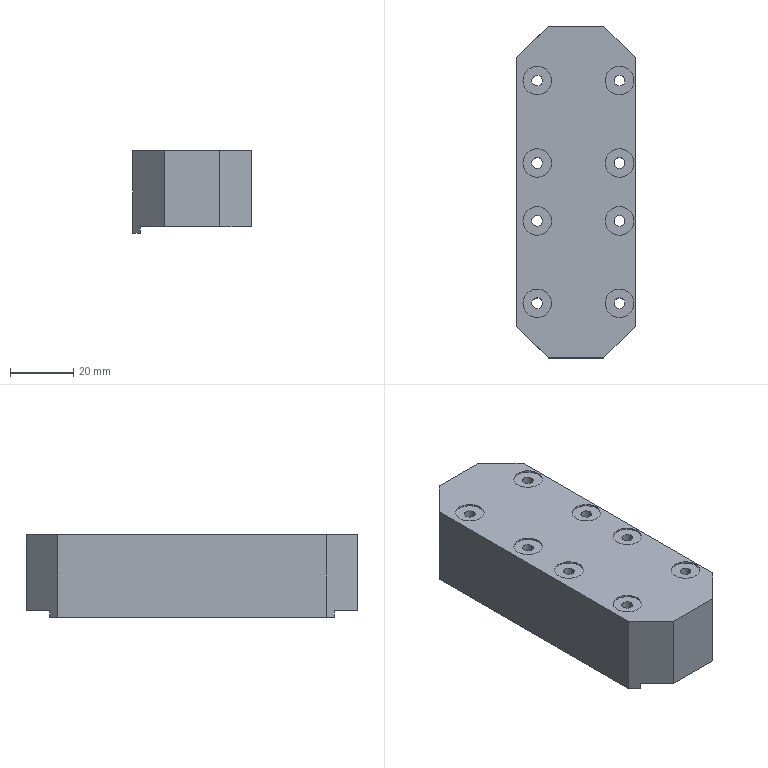Part | SolidWorks | features Chamfer 1, Cut 1, Extrusion 1, HoleWzd 1 | 1 solid | 52 faces | box 37.5 x 104.657 x 26 mm | volume 87866 mm3 | cylinder 32 | plane 20 | commonest cylinder face diameters 3.4 x16 9 x16
STEP:
#1=CARTESIAN_POINT('',(-17.5,32.7,23.5));
#2=VERTEX_POINT('',#1);
#3=CARTESIAN_POINT('',(-8.5,32.7,23.5));
#4=VERTEX_POINT('',#3);
#5=CARTESIAN_POINT('',(-13.,32.7,23.5));
#6=DIRECTION('',(0.,0.,1.));
#7=DIRECTION('',(1.,0.,0.));
#8=AXIS2_PLACEMENT_3D('',#5,#6,#7);
#9=CIRCLE('',#8,4.5);
#10=EDGE_CURVE('',#2,#4,#9,.T.);
#11=ORIENTED_EDGE('',*,*,#10,.F.);
#12=CARTESIAN_POINT('',(-17.5,32.7,24.));
#13=VERTEX_POINT('',#12);
#14=CARTESIAN_POINT('',(-17.5,32.7,24.));
#15=DIRECTION('',(0.,0.,1.));
#16=VECTOR('',#15,1000.);
#17=LINE('',#14,#16);
#18=EDGE_CURVE('',#2,#13,#17,.T.);
#19=ORIENTED_EDGE('',*,*,#18,.T.);
#20=CARTESIAN_POINT('',(-8.5,32.7,24.));
#21=VERTEX_POINT('',#20);
#22=CARTESIAN_POINT('',(-13.,32.7,24.));
#23=DIRECTION('',(0.,0.,1.));
#24=DIRECTION('',(1.,0.,0.));
#25=AXIS2_PLACEMENT_3D('',#22,#23,#24);
#26=CIRCLE('',#25,4.5);
#27=EDGE_CURVE('',#13,#21,#26,.T.);
#28=ORIENTED_EDGE('',*,*,#27,.T.);
#29=CARTESIAN_POINT('',(-8.5,32.7,24.));
#30=DIRECTION('',(0.,0.,1.));
#31=VECTOR('',#30,1000.);
#32=LINE('',#29,#31);
#33=EDGE_CURVE('',#4,#21,#32,.T.);
#34=ORIENTED_EDGE('',*,*,#33,.F.);
#35=EDGE_LOOP('',(#11,#19,#28,#34));
#36=FACE_OUTER_BOUND('',#35,.T.);
#37=CARTESIAN_POINT('',(-13.,32.7,24.));
#38=DIRECTION('',(0.,0.,1.));
#39=DIRECTION('',(1.,0.,0.));
#40=AXIS2_PLACEMENT_3D('',#37,#38,#39);
#41=CYLINDRICAL_SURFACE('',#40,4.5);
#42=ADVANCED_FACE('',(#36),#41,.F.);
#43=CARTESIAN_POINT('',(-14.7,32.7,0.));
#44=VERTEX_POINT('',#43);
#45=CARTESIAN_POINT('',(-11.3,32.7,0.));
#46=VERTEX_POINT('',#45);
#47=CARTESIAN_POINT('',(-13.,32.7,0.));
#48=DIRECTION('',(0.,0.,1.));
#49=DIRECTION('',(1.,0.,0.));
#50=AXIS2_PLACEMENT_3D('',#47,#48,#49);
#51=CIRCLE('',#50,1.7);
#52=EDGE_CURVE('',#44,#46,#51,.T.);
#53=ORIENTED_EDGE('',*,*,#52,.F.);
#54=CARTESIAN_POINT('',(-14.7,32.7,23.5));
#55=VERTEX_POINT('',#54);
#56=CARTESIAN_POINT('',(-14.7,32.7,24.));
#57=DIRECTION('',(0.,0.,1.));
#58=VECTOR('',#57,1000.);
#59=LINE('',#56,#58);
#60=EDGE_CURVE('',#44,#55,#59,.T.);
#61=ORIENTED_EDGE('',*,*,#60,.T.);
#62=CARTESIAN_POINT('',(-11.3,32.7,23.5));
#63=VERTEX_POINT('',#62);
#64=CARTESIAN_POINT('',(-13.,32.7,23.5));
#65=DIRECTION('',(0.,0.,1.));
#66=DIRECTION('',(1.,0.,0.));
#67=AXIS2_PLACEMENT_3D('',#64,#65,#66);
#68=CIRCLE('',#67,1.7);
#69=EDGE_CURVE('',#55,#63,#68,.T.);
#70=ORIENTED_EDGE('',*,*,#69,.T.);
#71=CARTESIAN_POINT('',(-11.3,32.7,24.));
#72=DIRECTION('',(0.,0.,1.));
#73=VECTOR('',#72,1000.);
#74=LINE('',#71,#73);
#75=EDGE_CURVE('',#46,#63,#74,.T.);
#76=ORIENTED_EDGE('',*,*,#75,.F.);
#77=EDGE_LOOP('',(#53,#61,#70,#76));
#78=FACE_OUTER_BOUND('',#77,.T.);
#79=CARTESIAN_POINT('',(-13.,32.7,24.));
#80=DIRECTION('',(0.,0.,1.));
#81=DIRECTION('',(1.,0.,0.));
#82=AXIS2_PLACEMENT_3D('',#79,#80,#81);
#83=CYLINDRICAL_SURFACE('',#82,1.7);
#84=ADVANCED_FACE('',(#78),#83,.F.);
#85=CARTESIAN_POINT('',(8.5,32.7,23.5));
#86=VERTEX_POINT('',#85);
#87=CARTESIAN_POINT('',(17.5,32.7,23.5));
#88=VERTEX_POINT('',#87);
#89=CARTESIAN_POINT('',(13.,32.7,23.5));
#90=DIRECTION('',(0.,0.,1.));
#91=DIRECTION('',(1.,0.,0.));
#92=AXIS2_PLACEMENT_3D('',#89,#90,#91);
#93=CIRCLE('',#92,4.5);
#94=EDGE_CURVE('',#86,#88,#93,.T.);
#95=ORIENTED_EDGE('',*,*,#94,.F.);
#96=CARTESIAN_POINT('',(8.5,32.7,24.));
#97=VERTEX_POINT('',#96);
#98=CARTESIAN_POINT('',(8.5,32.7,24.));
#99=DIRECTION('',(0.,0.,1.));
#100=VECTOR('',#99,1000.);
#101=LINE('',#98,#100);
#102=EDGE_CURVE('',#86,#97,#101,.T.);
#103=ORIENTED_EDGE('',*,*,#102,.T.);
#104=CARTESIAN_POINT('',(17.5,32.7,24.));
#105=VERTEX_POINT('',#104);
#106=CARTESIAN_POINT('',(13.,32.7,24.));
#107=DIRECTION('',(0.,0.,1.));
#108=DIRECTION('',(1.,0.,0.));
#109=AXIS2_PLACEMENT_3D('',#106,#107,#108);
#110=CIRCLE('',#109,4.5);
#111=EDGE_CURVE('',#97,#105,#110,.T.);
#112=ORIENTED_EDGE('',*,*,#111,.T.);
#113=CARTESIAN_POINT('',(17.5,32.7,24.));
#114=DIRECTION('',(0.,0.,1.));
#115=VECTOR('',#114,1000.);
#116=LINE('',#113,#115);
#117=EDGE_CURVE('',#88,#105,#116,.T.);
#118=ORIENTED_EDGE('',*,*,#117,.F.);
#119=EDGE_LOOP('',(#95,#103,#112,#118));
#120=FACE_OUTER_BOUND('',#119,.T.);
#121=CARTESIAN_POINT('',(13.,32.7,24.));
#122=DIRECTION('',(0.,0.,1.));
#123=DIRECTION('',(1.,0.,0.));
#124=AXIS2_PLACEMENT_3D('',#121,#122,#123);
#125=CYLINDRICAL_SURFACE('',#124,4.5);
#126=ADVANCED_FACE('',(#120),#125,.F.);
#127=CARTESIAN_POINT('',(11.3,32.7,0.));
#128=VERTEX_POINT('',#127);
#129=CARTESIAN_POINT('',(14.7,32.7,0.));
#130=VERTEX_POINT('',#129);
#131=CARTESIAN_POINT('',(13.,32.7,0.));
#132=DIRECTION('',(0.,0.,1.));
#133=DIRECTION('',(1.,0.,0.));
#134=AXIS2_PLACEMENT_3D('',#131,#132,#133);
#135=CIRCLE('',#134,1.7);
#136=EDGE_CURVE('',#128,#130,#135,.T.);
#137=ORIENTED_EDGE('',*,*,#136,.F.);
#138=CARTESIAN_POINT('',(11.3,32.7,23.5));
#139=VERTEX_POINT('',#138);
#140=CARTESIAN_POINT('',(11.3,32.7,24.));
#141=DIRECTION('',(0.,0.,1.));
#142=VECTOR('',#141,1000.);
#143=LINE('',#140,#142);
#144=EDGE_CURVE('',#128,#139,#143,.T.);
#145=ORIENTED_EDGE('',*,*,#144,.T.);
#146=CARTESIAN_POINT('',(14.7,32.7,23.5));
#147=VERTEX_POINT('',#146);
#148=CARTESIAN_POINT('',(13.,32.7,23.5));
#149=DIRECTION('',(0.,0.,1.));
#150=DIRECTION('',(1.,0.,0.));
#151=AXIS2_PLACEMENT_3D('',#148,#149,#150);
#152=CIRCLE('',#151,1.7);
#153=EDGE_CURVE('',#139,#147,#152,.T.);
#154=ORIENTED_EDGE('',*,*,#153,.T.);
#155=CARTESIAN_POINT('',(14.7,32.7,24.));
#156=DIRECTION('',(0.,0.,1.));
#157=VECTOR('',#156,1000.);
#158=LINE('',#155,#157);
#159=EDGE_CURVE('',#130,#147,#158,.T.);
#160=ORIENTED_EDGE('',*,*,#159,.F.);
#161=EDGE_LOOP('',(#137,#145,#154,#160));
#162=FACE_OUTER_BOUND('',#161,.T.);
#163=CARTESIAN_POINT('',(13.,32.7,24.));
#164=DIRECTION('',(0.,0.,1.));
#165=DIRECTION('',(1.,0.,0.));
#166=AXIS2_PLACEMENT_3D('',#163,#164,#165);
#167=CYLINDRICAL_SURFACE('',#166,1.7);
#168=ADVANCED_FACE('',(#162),#167,.F.);
#169=CARTESIAN_POINT('',(8.5,6.7,23.5));
#170=VERTEX_POINT('',#169);
#171=CARTESIAN_POINT('',(17.5,6.7,23.5));
#172=VERTEX_POINT('',#171);
#173=CARTESIAN_POINT('',(13.,6.7,23.5));
#174=DIRECTION('',(0.,0.,1.));
#175=DIRECTION('',(1.,0.,0.));
#176=AXIS2_PLACEMENT_3D('',#173,#174,#175);
#177=CIRCLE('',#176,4.5);
#178=EDGE_CURVE('',#170,#172,#177,.T.);
#179=ORIENTED_EDGE('',*,*,#178,.F.);
#180=CARTESIAN_POINT('',(8.5,6.7,24.));
#181=VERTEX_POINT('',#180);
#182=CARTESIAN_POINT('',(8.5,6.7,24.));
#183=DIRECTION('',(0.,0.,1.));
#184=VECTOR('',#183,1000.);
#185=LINE('',#182,#184);
#186=EDGE_CURVE('',#170,#181,#185,.T.);
#187=ORIENTED_EDGE('',*,*,#186,.T.);
#188=CARTESIAN_POINT('',(17.5,6.7,24.));
#189=VERTEX_POINT('',#188);
#190=CARTESIAN_POINT('',(13.,6.7,24.));
#191=DIRECTION('',(0.,0.,1.));
#192=DIRECTION('',(1.,0.,0.));
#193=AXIS2_PLACEMENT_3D('',#190,#191,#192);
#194=CIRCLE('',#193,4.5);
#195=EDGE_CURVE('',#181,#189,#194,.T.);
#196=ORIENTED_EDGE('',*,*,#195,.T.);
#197=CARTESIAN_POINT('',(17.5,6.7,24.));
#198=DIRECTION('',(0.,0.,1.));
#199=VECTOR('',#198,1000.);
#200=LINE('',#197,#199);
#201=EDGE_CURVE('',#172,#189,#200,.T.);
#202=ORIENTED_EDGE('',*,*,#201,.F.);
#203=EDGE_LOOP('',(#179,#187,#196,#202));
#204=FACE_OUTER_BOUND('',#203,.T.);
#205=CARTESIAN_POINT('',(13.,6.7,24.));
#206=DIRECTION('',(0.,0.,1.));
#207=DIRECTION('',(1.,0.,0.));
#208=AXIS2_PLACEMENT_3D('',#205,#206,#207);
#209=CYLINDRICAL_SURFACE('',#208,4.5);
#210=ADVANCED_FACE('',(#204),#209,.F.);
#211=CARTESIAN_POINT('',(11.3,6.7,0.));
#212=VERTEX_POINT('',#211);
#213=CARTESIAN_POINT('',(14.7,6.7,0.));
#214=VERTEX_POINT('',#213);
#215=CARTESIAN_POINT('',(13.,6.7,0.));
#216=DIRECTION('',(0.,0.,1.));
#217=DIRECTION('',(1.,0.,0.));
#218=AXIS2_PLACEMENT_3D('',#215,#216,#217);
#219=CIRCLE('',#218,1.7);
#220=EDGE_CURVE('',#212,#214,#219,.T.);
#221=ORIENTED_EDGE('',*,*,#220,.F.);
#222=CARTESIAN_POINT('',(11.3,6.7,23.5));
#223=VERTEX_POINT('',#222);
#224=CARTESIAN_POINT('',(11.3,6.7,24.));
#225=DIRECTION('',(0.,0.,1.));
#226=VECTOR('',#225,1000.);
#227=LINE('',#224,#226);
#228=EDGE_CURVE('',#212,#223,#227,.T.);
#229=ORIENTED_EDGE('',*,*,#228,.T.);
#230=CARTESIAN_POINT('',(14.7,6.7,23.5));
#231=VERTEX_POINT('',#230);
#232=CARTESIAN_POINT('',(13.,6.7,23.5));
#233=DIRECTION('',(0.,0.,1.));
#234=DIRECTION('',(1.,0.,0.));
#235=AXIS2_PLACEMENT_3D('',#232,#233,#234);
#236=CIRCLE('',#235,1.7);
#237=EDGE_CURVE('',#223,#231,#236,.T.);
#238=ORIENTED_EDGE('',*,*,#237,.T.);
#239=CARTESIAN_POINT('',(14.7,6.7,24.));
#240=DIRECTION('',(0.,0.,1.));
#241=VECTOR('',#240,1000.);
#242=LINE('',#239,#241);
#243=EDGE_CURVE('',#214,#231,#242,.T.);
#244=ORIENTED_EDGE('',*,*,#243,.F.);
#245=EDGE_LOOP('',(#221,#229,#238,#244));
#246=FACE_OUTER_BOUND('',#245,.T.);
#247=CARTESIAN_POINT('',(13.,6.7,24.));
#248=DIRECTION('',(0.,0.,1.));
#249=DIRECTION('',(1.,0.,0.));
#250=AXIS2_PLACEMENT_3D('',#247,#248,#249);
#251=CYLINDRICAL_SURFACE('',#250,1.7);
#252=ADVANCED_FACE('',(#246),#251,.F.);
#253=CARTESIAN_POINT('',(-17.5,6.7,23.5));
#254=VERTEX_POINT('',#253);
#255=CARTESIAN_POINT('',(-8.5,6.7,23.5));
#256=VERTEX_POINT('',#255);
#257=CARTESIAN_POINT('',(-13.,6.7,23.5));
#258=DIRECTION('',(0.,0.,1.));
#259=DIRECTION('',(1.,0.,0.));
#260=AXIS2_PLACEMENT_3D('',#257,#258,#259);
#261=CIRCLE('',#260,4.5);
#262=EDGE_CURVE('',#254,#256,#261,.T.);
#263=ORIENTED_EDGE('',*,*,#262,.F.);
#264=CARTESIAN_POINT('',(-17.5,6.7,24.));
#265=VERTEX_POINT('',#264);
#266=CARTESIAN_POINT('',(-17.5,6.7,24.));
#267=DIRECTION('',(0.,0.,1.));
#268=VECTOR('',#267,1000.);
#269=LINE('',#266,#268);
#270=EDGE_CURVE('',#254,#265,#269,.T.);
#271=ORIENTED_EDGE('',*,*,#270,.T.);
#272=CARTESIAN_POINT('',(-8.5,6.7,24.));
#273=VERTEX_POINT('',#272);
#274=CARTESIAN_POINT('',(-13.,6.7,24.));
#275=DIRECTION('',(0.,0.,1.));
#276=DIRECTION('',(1.,0.,0.));
#277=AXIS2_PLACEMENT_3D('',#274,#275,#276);
#278=CIRCLE('',#277,4.5);
#279=EDGE_CURVE('',#265,#273,#278,.T.);
#280=ORIENTED_EDGE('',*,*,#279,.T.);
#281=CARTESIAN_POINT('',(-8.5,6.7,24.));
#282=DIRECTION('',(0.,0.,1.));
#283=VECTOR('',#282,1000.);
#284=LINE('',#281,#283);
#285=EDGE_CURVE('',#256,#273,#284,.T.);
#286=ORIENTED_EDGE('',*,*,#285,.F.);
#287=EDGE_LOOP('',(#263,#271,#280,#286));
#288=FACE_OUTER_BOUND('',#287,.T.);
#289=CARTESIAN_POINT('',(-13.,6.7,24.));
#290=DIRECTION('',(0.,0.,1.));
#291=DIRECTION('',(1.,0.,0.));
#292=AXIS2_PLACEMENT_3D('',#289,#290,#291);
#293=CYLINDRICAL_SURFACE('',#292,4.5);
#294=ADVANCED_FACE('',(#288),#293,.F.);
#295=CARTESIAN_POINT('',(-14.7,6.7,0.));
#296=VERTEX_POINT('',#295);
#297=CARTESIAN_POINT('',(-11.3,6.7,0.));
#298=VERTEX_POINT('',#297);
#299=CARTESIAN_POINT('',(-13.,6.7,0.));
#300=DIRECTION('',(0.,0.,1.));
#301=DIRECTION('',(1.,0.,0.));
#302=AXIS2_PLACEMENT_3D('',#299,#300,#301);
#303=CIRCLE('',#302,1.7);
#304=EDGE_CURVE('',#296,#298,#303,.T.);
#305=ORIENTED_EDGE('',*,*,#304,.F.);
#306=CARTESIAN_POINT('',(-14.7,6.7,23.5));
#307=VERTEX_POINT('',#306);
#308=CARTESIAN_POINT('',(-14.7,6.7,24.));
#309=DIRECTION('',(0.,0.,1.));
#310=VECTOR('',#309,1000.);
#311=LINE('',#308,#310);
#312=EDGE_CURVE('',#296,#307,#311,.T.);
#313=ORIENTED_EDGE('',*,*,#312,.T.);
#314=CARTESIAN_POINT('',(-11.3,6.7,23.5));
#315=VERTEX_POINT('',#314);
#316=CARTESIAN_POINT('',(-13.,6.7,23.5));
#317=DIRECTION('',(0.,0.,1.));
#318=DIRECTION('',(1.,0.,0.));
#319=AXIS2_PLACEMENT_3D('',#316,#317,#318);
#320=CIRCLE('',#319,1.7);
#321=EDGE_CURVE('',#307,#315,#320,.T.);
#322=ORIENTED_EDGE('',*,*,#321,.T.);
#323=CARTESIAN_POINT('',(-11.3,6.7,24.));
#324=DIRECTION('',(0.,0.,1.));
#325=VECTOR('',#324,1000.);
#326=LINE('',#323,#325);
#327=EDGE_CURVE('',#298,#315,#326,.T.);
#328=ORIENTED_EDGE('',*,*,#327,.F.);
#329=EDGE_LOOP('',(#305,#313,#322,#328));
#330=FACE_OUTER_BOUND('',#329,.T.);
#331=CARTESIAN_POINT('',(-13.,6.7,24.));
#332=DIRECTION('',(0.,0.,1.));
#333=DIRECTION('',(1.,0.,0.));
#334=AXIS2_PLACEMENT_3D('',#331,#332,#333);
#335=CYLINDRICAL_SURFACE('',#334,1.7);
#336=ADVANCED_FACE('',(#330),#335,.F.);
#337=CARTESIAN_POINT('',(-17.5,-11.557,23.5));
#338=VERTEX_POINT('',#337);
#339=CARTESIAN_POINT('',(-8.5,-11.557,23.5));
#340=VERTEX_POINT('',#339);
#341=CARTESIAN_POINT('',(-13.,-11.557,23.5));
#342=DIRECTION('',(0.,0.,1.));
#343=DIRECTION('',(1.,0.,0.));
#344=AXIS2_PLACEMENT_3D('',#341,#342,#343);
#345=CIRCLE('',#344,4.5);
#346=EDGE_CURVE('',#338,#340,#345,.T.);
#347=ORIENTED_EDGE('',*,*,#346,.F.);
#348=CARTESIAN_POINT('',(-17.5,-11.557,24.));
#349=VERTEX_POINT('',#348);
#350=CARTESIAN_POINT('',(-17.5,-11.557,24.));
#351=DIRECTION('',(0.,0.,1.));
#352=VECTOR('',#351,1000.);
#353=LINE('',#350,#352);
#354=EDGE_CURVE('',#338,#349,#353,.T.);
#355=ORIENTED_EDGE('',*,*,#354,.T.);
#356=CARTESIAN_POINT('',(-8.5,-11.557,24.));
#357=VERTEX_POINT('',#356);
#358=CARTESIAN_POINT('',(-13.,-11.557,24.));
#359=DIRECTION('',(0.,0.,1.));
#360=DIRECTION('',(1.,0.,0.));
#361=AXIS2_PLACEMENT_3D('',#358,#359,#360);
#362=CIRCLE('',#361,4.5);
#363=EDGE_CURVE('',#349,#357,#362,.T.);
#364=ORIENTED_EDGE('',*,*,#363,.T.);
#365=CARTESIAN_POINT('',(-8.5,-11.557,24.));
#366=DIRECTION('',(0.,0.,1.));
#367=VECTOR('',#366,1000.);
#368=LINE('',#365,#367);
#369=EDGE_CURVE('',#340,#357,#368,.T.);
#370=ORIENTED_EDGE('',*,*,#369,.F.);
#371=EDGE_LOOP('',(#347,#355,#364,#370));
#372=FACE_OUTER_BOUND('',#371,.T.);
#373=CARTESIAN_POINT('',(-13.,-11.557,24.));
#374=DIRECTION('',(0.,0.,1.));
#375=DIRECTION('',(1.,0.,0.));
#376=AXIS2_PLACEMENT_3D('',#373,#374,#375);
#377=CYLINDRICAL_SURFACE('',#376,4.5);
#378=ADVANCED_FACE('',(#372),#377,.F.);
#379=CARTESIAN_POINT('',(-14.7,-11.557,0.));
#380=VERTEX_POINT('',#379);
#381=CARTESIAN_POINT('',(-11.3,-11.557,0.));
#382=VERTEX_POINT('',#381);
#383=CARTESIAN_POINT('',(-13.,-11.557,0.));
#384=DIRECTION('',(0.,0.,1.));
#385=DIRECTION('',(1.,0.,0.));
#386=AXIS2_PLACEMENT_3D('',#383,#384,#385);
#387=CIRCLE('',#386,1.7);
#388=EDGE_CURVE('',#380,#382,#387,.T.);
#389=ORIENTED_EDGE('',*,*,#388,.F.);
#390=CARTESIAN_POINT('',(-14.7,-11.557,23.5));
#391=VERTEX_POINT('',#390);
#392=CARTESIAN_POINT('',(-14.7,-11.557,24.));
#393=DIRECTION('',(0.,0.,1.));
#394=VECTOR('',#393,1000.);
#395=LINE('',#392,#394);
#396=EDGE_CURVE('',#380,#391,#395,.T.);
#397=ORIENTED_EDGE('',*,*,#396,.T.);
#398=CARTESIAN_POINT('',(-11.3,-11.557,23.5));
#399=VERTEX_POINT('',#398);
#400=CARTESIAN_POINT('',(-13.,-11.557,23.5));
#401=DIRECTION('',(0.,0.,1.));
#402=DIRECTION('',(1.,0.,0.));
#403=AXIS2_PLACEMENT_3D('',#400,#401,#402);
#404=CIRCLE('',#403,1.7);
#405=EDGE_CURVE('',#391,#399,#404,.T.);
#406=ORIENTED_EDGE('',*,*,#405,.T.);
#407=CARTESIAN_POINT('',(-11.3,-11.557,24.));
#408=DIRECTION('',(0.,0.,1.));
#409=VECTOR('',#408,1000.);
#410=LINE('',#407,#409);
#411=EDGE_CURVE('',#382,#399,#410,.T.);
#412=ORIENTED_EDGE('',*,*,#411,.F.);
#413=EDGE_LOOP('',(#389,#397,#406,#412));
#414=FACE_OUTER_BOUND('',#413,.T.);
#415=CARTESIAN_POINT('',(-13.,-11.557,24.));
#416=DIRECTION('',(0.,0.,1.));
#417=DIRECTION('',(1.,0.,0.));
#418=AXIS2_PLACEMENT_3D('',#415,#416,#417);
#419=CYLINDRICAL_SURFACE('',#418,1.7);
#420=ADVANCED_FACE('',(#414),#419,.F.);
#421=CARTESIAN_POINT('',(8.5,-11.557,23.5));
#422=VERTEX_POINT('',#421);
#423=CARTESIAN_POINT('',(17.5,-11.557,23.5));
#424=VERTEX_POINT('',#423);
#425=CARTESIAN_POINT('',(13.,-11.557,23.5));
#426=DIRECTION('',(0.,0.,1.));
#427=DIRECTION('',(1.,0.,0.));
#428=AXIS2_PLACEMENT_3D('',#425,#426,#427);
#429=CIRCLE('',#428,4.5);
#430=EDGE_CURVE('',#422,#424,#429,.T.);
#431=ORIENTED_EDGE('',*,*,#430,.F.);
#432=CARTESIAN_POINT('',(8.5,-11.557,24.));
#433=VERTEX_POINT('',#432);
#434=CARTESIAN_POINT('',(8.5,-11.557,24.));
#435=DIRECTION('',(0.,0.,1.));
#436=VECTOR('',#435,1000.);
#437=LINE('',#434,#436);
#438=EDGE_CURVE('',#422,#433,#437,.T.);
#439=ORIENTED_EDGE('',*,*,#438,.T.);
#440=CARTESIAN_POINT('',(17.5,-11.557,24.));
#441=VERTEX_POINT('',#440);
#442=CARTESIAN_POINT('',(13.,-11.557,24.));
#443=DIRECTION('',(0.,0.,1.));
#444=DIRECTION('',(1.,0.,0.));
#445=AXIS2_PLACEMENT_3D('',#442,#443,#444);
#446=CIRCLE('',#445,4.5);
#447=EDGE_CURVE('',#433,#441,#446,.T.);
#448=ORIENTED_EDGE('',*,*,#447,.T.);
#449=CARTESIAN_POINT('',(17.5,-11.557,24.));
#450=DIRECTION('',(0.,0.,1.));
#451=VECTOR('',#450,1000.);
#452=LINE('',#449,#451);
#453=EDGE_CURVE('',#424,#441,#452,.T.);
#454=ORIENTED_EDGE('',*,*,#453,.F.);
#455=EDGE_LOOP('',(#431,#439,#448,#454));
#456=FACE_OUTER_BOUND('',#455,.T.);
#457=CARTESIAN_POINT('',(13.,-11.557,24.));
#458=DIRECTION('',(0.,0.,1.));
#459=DIRECTION('',(1.,0.,0.));
#460=AXIS2_PLACEMENT_3D('',#457,#458,#459);
#461=CYLINDRICAL_SURFACE('',#460,4.5);
#462=ADVANCED_FACE('',(#456),#461,.F.);
#463=CARTESIAN_POINT('',(11.3,-11.557,0.));
#464=VERTEX_POINT('',#463);
#465=CARTESIAN_POINT('',(14.7,-11.557,0.));
#466=VERTEX_POINT('',#465);
#467=CARTESIAN_POINT('',(13.,-11.557,0.));
#468=DIRECTION('',(0.,0.,1.));
#469=DIRECTION('',(1.,0.,0.));
#470=AXIS2_PLACEMENT_3D('',#467,#468,#469);
#471=CIRCLE('',#470,1.7);
#472=EDGE_CURVE('',#464,#466,#471,.T.);
#473=ORIENTED_EDGE('',*,*,#472,.F.);
#474=CARTESIAN_POINT('',(11.3,-11.557,23.5));
#475=VERTEX_POINT('',#474);
#476=CARTESIAN_POINT('',(11.3,-11.557,24.));
#477=DIRECTION('',(0.,0.,1.));
#478=VECTOR('',#477,1000.);
#479=LINE('',#476,#478);
#480=EDGE_CURVE('',#464,#475,#479,.T.);
#481=ORIENTED_EDGE('',*,*,#480,.T.);
#482=CARTESIAN_POINT('',(14.7,-11.557,23.5));
#483=VERTEX_POINT('',#482);
#484=CARTESIAN_POINT('',(13.,-11.557,23.5));
#485=DIRECTION('',(0.,0.,1.));
#486=DIRECTION('',(1.,0.,0.));
#487=AXIS2_PLACEMENT_3D('',#484,#485,#486);
#488=CIRCLE('',#487,1.7);
#489=EDGE_CURVE('',#475,#483,#488,.T.);
#490=ORIENTED_EDGE('',*,*,#489,.T.);
#491=CARTESIAN_POINT('',(14.7,-11.557,24.));
#492=DIRECTION('',(0.,0.,1.));
#493=VECTOR('',#492,1000.);
#494=LINE('',#491,#493);
#495=EDGE_CURVE('',#466,#483,#494,.T.);
#496=ORIENTED_EDGE('',*,*,#495,.F.);
#497=EDGE_LOOP('',(#473,#481,#490,#496));
#498=FACE_OUTER_BOUND('',#497,.T.);
#499=CARTESIAN_POINT('',(13.,-11.557,24.));
#500=DIRECTION('',(0.,0.,1.));
#501=DIRECTION('',(1.,0.,0.));
#502=AXIS2_PLACEMENT_3D('',#499,#500,#501);
#503=CYLINDRICAL_SURFACE('',#502,1.7);
#504=ADVANCED_FACE('',(#498),#503,.F.);
#505=CARTESIAN_POINT('',(8.5,-37.557,23.5));
#506=VERTEX_POINT('',#505);
#507=CARTESIAN_POINT('',(17.5,-37.557,23.5));
#508=VERTEX_POINT('',#507);
#509=CARTESIAN_POINT('',(13.,-37.557,23.5));
#510=DIRECTION('',(0.,0.,1.));
#511=DIRECTION('',(1.,0.,0.));
#512=AXIS2_PLACEMENT_3D('',#509,#510,#511);
#513=CIRCLE('',#512,4.5);
#514=EDGE_CURVE('',#506,#508,#513,.T.);
#515=ORIENTED_EDGE('',*,*,#514,.F.);
#516=CARTESIAN_POINT('',(8.5,-37.557,24.));
#517=VERTEX_POINT('',#516);
#518=CARTESIAN_POINT('',(8.5,-37.557,24.));
#519=DIRECTION('',(0.,0.,1.));
#520=VECTOR('',#519,1000.);
#521=LINE('',#518,#520);
#522=EDGE_CURVE('',#506,#517,#521,.T.);
#523=ORIENTED_EDGE('',*,*,#522,.T.);
#524=CARTESIAN_POINT('',(17.5,-37.557,24.));
#525=VERTEX_POINT('',#524);
#526=CARTESIAN_POINT('',(13.,-37.557,24.));
#527=DIRECTION('',(0.,0.,1.));
#528=DIRECTION('',(1.,0.,0.));
#529=AXIS2_PLACEMENT_3D('',#526,#527,#528);
#530=CIRCLE('',#529,4.5);
#531=EDGE_CURVE('',#517,#525,#530,.T.);
#532=ORIENTED_EDGE('',*,*,#531,.T.);
#533=CARTESIAN_POINT('',(17.5,-37.557,24.));
#534=DIRECTION('',(0.,0.,1.));
#535=VECTOR('',#534,1000.);
#536=LINE('',#533,#535);
#537=EDGE_CURVE('',#508,#525,#536,.T.);
#538=ORIENTED_EDGE('',*,*,#537,.F.);
#539=EDGE_LOOP('',(#515,#523,#532,#538));
#540=FACE_OUTER_BOUND('',#539,.T.);
#541=CARTESIAN_POINT('',(13.,-37.557,24.));
#542=DIRECTION('',(0.,0.,1.));
#543=DIRECTION('',(1.,0.,0.));
#544=AXIS2_PLACEMENT_3D('',#541,#542,#543);
#545=CYLINDRICAL_SURFACE('',#544,4.5);
#546=ADVANCED_FACE('',(#540),#545,.F.);
#547=CARTESIAN_POINT('',(11.3,-37.557,0.));
#548=VERTEX_POINT('',#547);
#549=CARTESIAN_POINT('',(14.7,-37.557,0.));
#550=VERTEX_POINT('',#549);
#551=CARTESIAN_POINT('',(13.,-37.557,0.));
#552=DIRECTION('',(0.,0.,1.));
#553=DIRECTION('',(1.,0.,0.));
#554=AXIS2_PLACEMENT_3D('',#551,#552,#553);
#555=CIRCLE('',#554,1.7);
#556=EDGE_CURVE('',#548,#550,#555,.T.);
#557=ORIENTED_EDGE('',*,*,#556,.F.);
#558=CARTESIAN_POINT('',(11.3,-37.557,23.5));
#559=VERTEX_POINT('',#558);
#560=CARTESIAN_POINT('',(11.3,-37.557,24.));
#561=DIRECTION('',(0.,0.,1.));
#562=VECTOR('',#561,1000.);
#563=LINE('',#560,#562);
#564=EDGE_CURVE('',#548,#559,#563,.T.);
#565=ORIENTED_EDGE('',*,*,#564,.T.);
#566=CARTESIAN_POINT('',(14.7,-37.557,23.5));
#567=VERTEX_POINT('',#566);
#568=CARTESIAN_POINT('',(13.,-37.557,23.5));
#569=DIRECTION('',(0.,0.,1.));
#570=DIRECTION('',(1.,0.,0.));
#571=AXIS2_PLACEMENT_3D('',#568,#569,#570);
#572=CIRCLE('',#571,1.7);
#573=EDGE_CURVE('',#559,#567,#572,.T.);
#574=ORIENTED_EDGE('',*,*,#573,.T.);
#575=CARTESIAN_POINT('',(14.7,-37.557,24.));
#576=DIRECTION('',(0.,0.,1.));
#577=VECTOR('',#576,1000.);
#578=LINE('',#575,#577);
#579=EDGE_CURVE('',#550,#567,#578,.T.);
#580=ORIENTED_EDGE('',*,*,#579,.F.);
#581=EDGE_LOOP('',(#557,#565,#574,#580));
#582=FACE_OUTER_BOUND('',#581,.T.);
#583=CARTESIAN_POINT('',(13.,-37.557,24.));
#584=DIRECTION('',(0.,0.,1.));
#585=DIRECTION('',(1.,0.,0.));
#586=AXIS2_PLACEMENT_3D('',#583,#584,#585);
#587=CYLINDRICAL_SURFACE('',#586,1.7);
#588=ADVANCED_FACE('',(#582),#587,.F.);
#589=CARTESIAN_POINT('',(-17.5,-37.557,23.5));
#590=VERTEX_POINT('',#589);
#591=CARTESIAN_POINT('',(-8.5,-37.557,23.5));
#592=VERTEX_POINT('',#591);
#593=CARTESIAN_POINT('',(-13.,-37.557,23.5));
#594=DIRECTION('',(0.,0.,1.));
#595=DIRECTION('',(1.,0.,0.));
#596=AXIS2_PLACEMENT_3D('',#593,#594,#595);
#597=CIRCLE('',#596,4.5);
#598=EDGE_CURVE('',#590,#592,#597,.T.);
#599=ORIENTED_EDGE('',*,*,#598,.F.);
#600=CARTESIAN_POINT('',(-17.5,-37.557,24.));
#601=VERTEX_POINT('',#600);
#602=CARTESIAN_POINT('',(-17.5,-37.557,24.));
#603=DIRECTION('',(0.,0.,1.));
#604=VECTOR('',#603,1000.);
#605=LINE('',#602,#604);
#606=EDGE_CURVE('',#590,#601,#605,.T.);
#607=ORIENTED_EDGE('',*,*,#606,.T.);
#608=CARTESIAN_POINT('',(-8.5,-37.557,24.));
#609=VERTEX_POINT('',#608);
#610=CARTESIAN_POINT('',(-13.,-37.557,24.));
#611=DIRECTION('',(0.,0.,1.));
#612=DIRECTION('',(1.,0.,0.));
#613=AXIS2_PLACEMENT_3D('',#610,#611,#612);
#614=CIRCLE('',#613,4.5);
#615=EDGE_CURVE('',#601,#609,#614,.T.);
#616=ORIENTED_EDGE('',*,*,#615,.T.);
#617=CARTESIAN_POINT('',(-8.5,-37.557,24.));
#618=DIRECTION('',(0.,0.,1.));
#619=VECTOR('',#618,1000.);
#620=LINE('',#617,#619);
#621=EDGE_CURVE('',#592,#609,#620,.T.);
#622=ORIENTED_EDGE('',*,*,#621,.F.);
#623=EDGE_LOOP('',(#599,#607,#616,#622));
#624=FACE_OUTER_BOUND('',#623,.T.);
#625=CARTESIAN_POINT('',(-13.,-37.557,24.));
#626=DIRECTION('',(0.,0.,1.));
#627=DIRECTION('',(1.,0.,0.));
#628=AXIS2_PLACEMENT_3D('',#625,#626,#627);
#629=CYLINDRICAL_SURFACE('',#628,4.5);
#630=ADVANCED_FACE('',(#624),#629,.F.);
#631=CARTESIAN_POINT('',(-14.7,-37.557,0.));
#632=VERTEX_POINT('',#631);
#633=CARTESIAN_POINT('',(-11.3,-37.557,0.));
#634=VERTEX_POINT('',#633);
#635=CARTESIAN_POINT('',(-13.,-37.557,0.));
#636=DIRECTION('',(0.,0.,1.));
#637=DIRECTION('',(1.,0.,0.));
#638=AXIS2_PLACEMENT_3D('',#635,#636,#637);
#639=CIRCLE('',#638,1.7);
#640=EDGE_CURVE('',#632,#634,#639,.T.);
#641=ORIENTED_EDGE('',*,*,#640,.F.);
#642=CARTESIAN_POINT('',(-14.7,-37.557,23.5));
#643=VERTEX_POINT('',#642);
#644=CARTESIAN_POINT('',(-14.7,-37.557,24.));
#645=DIRECTION('',(0.,0.,1.));
#646=VECTOR('',#645,1000.);
#647=LINE('',#644,#646);
#648=EDGE_CURVE('',#632,#643,#647,.T.);
#649=ORIENTED_EDGE('',*,*,#648,.T.);
#650=CARTESIAN_POINT('',(-11.3,-37.557,23.5));
#651=VERTEX_POINT('',#650);
#652=CARTESIAN_POINT('',(-13.,-37.557,23.5));
#653=DIRECTION('',(0.,0.,1.));
#654=DIRECTION('',(1.,0.,0.));
#655=AXIS2_PLACEMENT_3D('',#652,#653,#654);
#656=CIRCLE('',#655,1.7);
#657=EDGE_CURVE('',#643,#651,#656,.T.);
#658=ORIENTED_EDGE('',*,*,#657,.T.);
#659=CARTESIAN_POINT('',(-11.3,-37.557,24.));
#660=DIRECTION('',(0.,0.,1.));
#661=VECTOR('',#660,1000.);
#662=LINE('',#659,#661);
#663=EDGE_CURVE('',#634,#651,#662,.T.);
#664=ORIENTED_EDGE('',*,*,#663,.F.);
#665=EDGE_LOOP('',(#641,#649,#658,#664));
#666=FACE_OUTER_BOUND('',#665,.T.);
#667=CARTESIAN_POINT('',(-13.,-37.557,24.));
#668=DIRECTION('',(0.,0.,1.));
#669=DIRECTION('',(1.,0.,0.));
#670=AXIS2_PLACEMENT_3D('',#667,#668,#669);
#671=CYLINDRICAL_SURFACE('',#670,1.7);
#672=ADVANCED_FACE('',(#666),#671,.F.);
#673=CARTESIAN_POINT('',(-19.5,39.9,-2.));
#674=VERTEX_POINT('',#673);
#675=CARTESIAN_POINT('',(-19.5,-44.757,-2.));
#676=VERTEX_POINT('',#675);
#677=CARTESIAN_POINT('',(-19.5,49.9,-2.));
#678=DIRECTION('',(0.,-1.,0.));
#679=VECTOR('',#678,1000.);
#680=LINE('',#677,#679);
#681=EDGE_CURVE('',#674,#676,#680,.T.);
#682=ORIENTED_EDGE('',*,*,#681,.T.);
#683=CARTESIAN_POINT('',(-19.5,-44.757,24.));
#684=VERTEX_POINT('',#683);
#685=CARTESIAN_POINT('',(-19.5,-44.757,-2.));
#686=DIRECTION('',(0.,0.,1.));
#687=VECTOR('',#686,1000.);
#688=LINE('',#685,#687);
#689=EDGE_CURVE('',#676,#684,#688,.T.);
#690=ORIENTED_EDGE('',*,*,#689,.T.);
#691=CARTESIAN_POINT('',(-19.5,39.9,24.));
#692=VERTEX_POINT('',#691);
#693=CARTESIAN_POINT('',(-19.5,49.9,24.));
#694=DIRECTION('',(0.,-1.,0.));
#695=VECTOR('',#694,1000.);
#696=LINE('',#693,#695);
#697=EDGE_CURVE('',#692,#684,#696,.T.);
#698=ORIENTED_EDGE('',*,*,#697,.F.);
#699=CARTESIAN_POINT('',(-19.5,39.9,-2.));
#700=DIRECTION('',(0.,0.,-1.));
#701=VECTOR('',#700,1000.);
#702=LINE('',#699,#701);
#703=EDGE_CURVE('',#692,#674,#702,.T.);
#704=ORIENTED_EDGE('',*,*,#703,.T.);
#705=EDGE_LOOP('',(#682,#690,#698,#704));
#706=FACE_OUTER_BOUND('',#705,.T.);
#707=CARTESIAN_POINT('',(-19.5,49.9,-2.));
#708=DIRECTION('',(-1.,0.,0.));
#709=DIRECTION('',(0.,-1.,0.));
#710=AXIS2_PLACEMENT_3D('',#707,#708,#709);
#711=PLANE('',#710);
#712=ADVANCED_FACE('',(#706),#711,.T.);
#713=CARTESIAN_POINT('',(8.,49.9,24.));
#714=VERTEX_POINT('',#713);
#715=CARTESIAN_POINT('',(-9.5,49.9,24.));
#716=VERTEX_POINT('',#715);
#717=CARTESIAN_POINT('',(-19.5,49.9,24.));
#718=DIRECTION('',(-1.,0.,0.));
#719=VECTOR('',#718,1000.);
#720=LINE('',#717,#719);
#721=EDGE_CURVE('',#714,#716,#720,.T.);
#722=ORIENTED_EDGE('',*,*,#721,.F.);
#723=CARTESIAN_POINT('',(8.,49.9,0.));
#724=VERTEX_POINT('',#723);
#725=CARTESIAN_POINT('',(8.,49.9,-2.));
#726=DIRECTION('',(0.,0.,-1.));
#727=VECTOR('',#726,1000.);
#728=LINE('',#725,#727);
#729=EDGE_CURVE('',#714,#724,#728,.T.);
#730=ORIENTED_EDGE('',*,*,#729,.T.);
#731=CARTESIAN_POINT('',(-9.5,49.9,0.));
#732=VERTEX_POINT('',#731);
#733=CARTESIAN_POINT('',(18.,49.9,0.));
#734=DIRECTION('',(-1.,0.,0.));
#735=VECTOR('',#734,1000.);
#736=LINE('',#733,#735);
#737=EDGE_CURVE('',#724,#732,#736,.T.);
#738=ORIENTED_EDGE('',*,*,#737,.T.);
#739=CARTESIAN_POINT('',(-9.5,49.9,-2.));
#740=DIRECTION('',(0.,0.,1.));
#741=VECTOR('',#740,1000.);
#742=LINE('',#739,#741);
#743=EDGE_CURVE('',#732,#716,#742,.T.);
#744=ORIENTED_EDGE('',*,*,#743,.T.);
#745=EDGE_LOOP('',(#722,#730,#738,#744));
#746=FACE_OUTER_BOUND('',#745,.T.);
#747=CARTESIAN_POINT('',(-19.5,49.9,-2.));
#748=DIRECTION('',(0.,1.,0.));
#749=DIRECTION('',(0.,0.,1.));
#750=AXIS2_PLACEMENT_3D('',#747,#748,#749);
#751=PLANE('',#750);
#752=ADVANCED_FACE('',(#746),#751,.T.);
#753=CARTESIAN_POINT('',(18.,-44.757,24.));
#754=VERTEX_POINT('',#753);
#755=CARTESIAN_POINT('',(18.,39.9,24.));
#756=VERTEX_POINT('',#755);
#757=CARTESIAN_POINT('',(18.,49.9,24.));
#758=DIRECTION('',(0.,1.,0.));
#759=VECTOR('',#758,1000.);
#760=LINE('',#757,#759);
#761=EDGE_CURVE('',#754,#756,#760,.T.);
#762=ORIENTED_EDGE('',*,*,#761,.F.);
#763=CARTESIAN_POINT('',(18.,-44.757,0.));
#764=VERTEX_POINT('',#763);
#765=CARTESIAN_POINT('',(18.,-44.757,-2.));
#766=DIRECTION('',(0.,0.,-1.));
#767=VECTOR('',#766,1000.);
#768=LINE('',#765,#767);
#769=EDGE_CURVE('',#754,#764,#768,.T.);
#770=ORIENTED_EDGE('',*,*,#769,.T.);
#771=CARTESIAN_POINT('',(18.,39.9,0.));
#772=VERTEX_POINT('',#771);
#773=CARTESIAN_POINT('',(18.,49.9,0.));
#774=DIRECTION('',(0.,-1.,0.));
#775=VECTOR('',#774,1000.);
#776=LINE('',#773,#775);
#777=EDGE_CURVE('',#772,#764,#776,.T.);
#778=ORIENTED_EDGE('',*,*,#777,.F.);
#779=CARTESIAN_POINT('',(18.,39.9,-2.));
#780=DIRECTION('',(0.,0.,1.));
#781=VECTOR('',#780,1000.);
#782=LINE('',#779,#781);
#783=EDGE_CURVE('',#772,#756,#782,.T.);
#784=ORIENTED_EDGE('',*,*,#783,.T.);
#785=EDGE_LOOP('',(#762,#770,#778,#784));
#786=FACE_OUTER_BOUND('',#785,.T.);
#787=CARTESIAN_POINT('',(18.,49.9,-2.));
#788=DIRECTION('',(1.,0.,0.));
#789=DIRECTION('',(0.,1.,0.));
#790=AXIS2_PLACEMENT_3D('',#787,#788,#789);
#791=PLANE('',#790);
#792=ADVANCED_FACE('',(#786),#791,.T.);
#793=CARTESIAN_POINT('',(8.,-54.757,0.));
#794=VERTEX_POINT('',#793);
#795=CARTESIAN_POINT('',(-9.5,-54.757,0.));
#796=VERTEX_POINT('',#795);
#797=CARTESIAN_POINT('',(18.,-54.757,0.));
#798=DIRECTION('',(-1.,0.,0.));
#799=VECTOR('',#798,1000.);
#800=LINE('',#797,#799);
#801=EDGE_CURVE('',#794,#796,#800,.T.);
#802=ORIENTED_EDGE('',*,*,#801,.F.);
#803=CARTESIAN_POINT('',(8.,-54.757,24.));
#804=VERTEX_POINT('',#803);
#805=CARTESIAN_POINT('',(8.,-54.757,-2.));
#806=DIRECTION('',(0.,0.,1.));
#807=VECTOR('',#806,1000.);
#808=LINE('',#805,#807);
#809=EDGE_CURVE('',#794,#804,#808,.T.);
#810=ORIENTED_EDGE('',*,*,#809,.T.);
#811=CARTESIAN_POINT('',(-9.5,-54.757,24.));
#812=VERTEX_POINT('',#811);
#813=CARTESIAN_POINT('',(-19.5,-54.757,24.));
#814=DIRECTION('',(1.,0.,0.));
#815=VECTOR('',#814,1000.);
#816=LINE('',#813,#815);
#817=EDGE_CURVE('',#812,#804,#816,.T.);
#818=ORIENTED_EDGE('',*,*,#817,.F.);
#819=CARTESIAN_POINT('',(-9.5,-54.757,-2.));
#820=DIRECTION('',(0.,0.,-1.));
#821=VECTOR('',#820,1000.);
#822=LINE('',#819,#821);
#823=EDGE_CURVE('',#812,#796,#822,.T.);
#824=ORIENTED_EDGE('',*,*,#823,.T.);
#825=EDGE_LOOP('',(#802,#810,#818,#824));
#826=FACE_OUTER_BOUND('',#825,.T.);
#827=CARTESIAN_POINT('',(-19.5,-54.757,-2.));
#828=DIRECTION('',(0.,-1.,0.));
#829=DIRECTION('',(0.,0.,-1.));
#830=AXIS2_PLACEMENT_3D('',#827,#828,#829);
#831=PLANE('',#830);
#832=ADVANCED_FACE('',(#826),#831,.T.);
#833=CARTESIAN_POINT('',(-17.,42.4,-2.));
#834=VERTEX_POINT('',#833);
#835=CARTESIAN_POINT('',(-17.,-47.257,-2.));
#836=VERTEX_POINT('',#835);
#837=CARTESIAN_POINT('',(-17.,49.9,-2.));
#838=DIRECTION('',(0.,-1.,0.));
#839=VECTOR('',#838,1000.);
#840=LINE('',#837,#839);
#841=EDGE_CURVE('',#834,#836,#840,.T.);
#842=ORIENTED_EDGE('',*,*,#841,.T.);
#843=CARTESIAN_POINT('',(-19.5,-44.757,-2.));
#844=DIRECTION('',(-0.7071,0.7071,0.));
#845=VECTOR('',#844,1000.);
#846=LINE('',#843,#845);
#847=EDGE_CURVE('',#836,#676,#846,.T.);
#848=ORIENTED_EDGE('',*,*,#847,.T.);
#849=ORIENTED_EDGE('',*,*,#681,.F.);
#850=CARTESIAN_POINT('',(-9.5,49.9,-2.));
#851=DIRECTION('',(0.7071,0.7071,0.));
#852=VECTOR('',#851,1000.);
#853=LINE('',#850,#852);
#854=EDGE_CURVE('',#674,#834,#853,.T.);
#855=ORIENTED_EDGE('',*,*,#854,.T.);
#856=EDGE_LOOP('',(#842,#848,#849,#855));
#857=FACE_OUTER_BOUND('',#856,.T.);
#858=CARTESIAN_POINT('',(0.,0.,-2.));
#859=DIRECTION('',(0.,0.,1.));
#860=DIRECTION('',(1.,0.,0.));
#861=AXIS2_PLACEMENT_3D('',#858,#859,#860);
#862=PLANE('',#861);
#863=ADVANCED_FACE('',(#857),#862,.F.);
#864=CARTESIAN_POINT('',(-13.,32.7,24.));
#865=DIRECTION('',(0.,0.,1.));
#866=DIRECTION('',(1.,0.,0.));
#867=AXIS2_PLACEMENT_3D('',#864,#865,#866);
#868=CIRCLE('',#867,4.5);
#869=EDGE_CURVE('',#21,#13,#868,.T.);
#870=ORIENTED_EDGE('',*,*,#869,.F.);
#871=ORIENTED_EDGE('',*,*,#27,.F.);
#872=EDGE_LOOP('',(#870,#871));
#873=FACE_BOUND('',#872,.T.);
#874=CARTESIAN_POINT('',(13.,32.7,24.));
#875=DIRECTION('',(0.,0.,1.));
#876=DIRECTION('',(1.,0.,0.));
#877=AXIS2_PLACEMENT_3D('',#874,#875,#876);
#878=CIRCLE('',#877,4.5);
#879=EDGE_CURVE('',#105,#97,#878,.T.);
#880=ORIENTED_EDGE('',*,*,#879,.F.);
#881=ORIENTED_EDGE('',*,*,#111,.F.);
#882=EDGE_LOOP('',(#880,#881));
#883=FACE_BOUND('',#882,.T.);
#884=CARTESIAN_POINT('',(13.,6.7,24.));
#885=DIRECTION('',(0.,0.,1.));
#886=DIRECTION('',(1.,0.,0.));
#887=AXIS2_PLACEMENT_3D('',#884,#885,#886);
#888=CIRCLE('',#887,4.5);
#889=EDGE_CURVE('',#189,#181,#888,.T.);
#890=ORIENTED_EDGE('',*,*,#889,.F.);
#891=ORIENTED_EDGE('',*,*,#195,.F.);
#892=EDGE_LOOP('',(#890,#891));
#893=FACE_BOUND('',#892,.T.);
#894=CARTESIAN_POINT('',(-13.,6.7,24.));
#895=DIRECTION('',(0.,0.,1.));
#896=DIRECTION('',(1.,0.,0.));
#897=AXIS2_PLACEMENT_3D('',#894,#895,#896);
#898=CIRCLE('',#897,4.5);
#899=EDGE_CURVE('',#273,#265,#898,.T.);
#900=ORIENTED_EDGE('',*,*,#899,.F.);
#901=ORIENTED_EDGE('',*,*,#279,.F.);
#902=EDGE_LOOP('',(#900,#901));
#903=FACE_BOUND('',#902,.T.);
#904=CARTESIAN_POINT('',(-13.,-11.557,24.));
#905=DIRECTION('',(0.,0.,1.));
#906=DIRECTION('',(1.,0.,0.));
#907=AXIS2_PLACEMENT_3D('',#904,#905,#906);
#908=CIRCLE('',#907,4.5);
#909=EDGE_CURVE('',#357,#349,#908,.T.);
#910=ORIENTED_EDGE('',*,*,#909,.F.);
#911=ORIENTED_EDGE('',*,*,#363,.F.);
#912=EDGE_LOOP('',(#910,#911));
#913=FACE_BOUND('',#912,.T.);
#914=CARTESIAN_POINT('',(13.,-11.557,24.));
#915=DIRECTION('',(0.,0.,1.));
#916=DIRECTION('',(1.,0.,0.));
#917=AXIS2_PLACEMENT_3D('',#914,#915,#916);
#918=CIRCLE('',#917,4.5);
#919=EDGE_CURVE('',#441,#433,#918,.T.);
#920=ORIENTED_EDGE('',*,*,#919,.F.);
#921=ORIENTED_EDGE('',*,*,#447,.F.);
#922=EDGE_LOOP('',(#920,#921));
#923=FACE_BOUND('',#922,.T.);
#924=CARTESIAN_POINT('',(13.,-37.557,24.));
#925=DIRECTION('',(0.,0.,1.));
#926=DIRECTION('',(1.,0.,0.));
#927=AXIS2_PLACEMENT_3D('',#924,#925,#926);
#928=CIRCLE('',#927,4.5);
#929=EDGE_CURVE('',#525,#517,#928,.T.);
#930=ORIENTED_EDGE('',*,*,#929,.F.);
#931=ORIENTED_EDGE('',*,*,#531,.F.);
#932=EDGE_LOOP('',(#930,#931));
#933=FACE_BOUND('',#932,.T.);
#934=CARTESIAN_POINT('',(-13.,-37.557,24.));
#935=DIRECTION('',(0.,0.,1.));
#936=DIRECTION('',(1.,0.,0.));
#937=AXIS2_PLACEMENT_3D('',#934,#935,#936);
#938=CIRCLE('',#937,4.5);
#939=EDGE_CURVE('',#609,#601,#938,.T.);
#940=ORIENTED_EDGE('',*,*,#939,.F.);
#941=ORIENTED_EDGE('',*,*,#615,.F.);
#942=EDGE_LOOP('',(#940,#941));
#943=FACE_BOUND('',#942,.T.);
#944=ORIENTED_EDGE('',*,*,#817,.T.);
#945=CARTESIAN_POINT('',(31.379,-31.379,24.));
#946=DIRECTION('',(0.7071,0.7071,0.));
#947=VECTOR('',#946,1000.);
#948=LINE('',#945,#947);
#949=EDGE_CURVE('',#804,#754,#948,.T.);
#950=ORIENTED_EDGE('',*,*,#949,.T.);
#951=ORIENTED_EDGE('',*,*,#761,.T.);
#952=CARTESIAN_POINT('',(28.95,28.95,24.));
#953=DIRECTION('',(-0.7071,0.7071,0.));
#954=VECTOR('',#953,1000.);
#955=LINE('',#952,#954);
#956=EDGE_CURVE('',#756,#714,#955,.T.);
#957=ORIENTED_EDGE('',*,*,#956,.T.);
#958=ORIENTED_EDGE('',*,*,#721,.T.);
#959=CARTESIAN_POINT('',(-29.7,29.7,24.));
#960=DIRECTION('',(-0.7071,-0.7071,0.));
#961=VECTOR('',#960,1000.);
#962=LINE('',#959,#961);
#963=EDGE_CURVE('',#716,#692,#962,.T.);
#964=ORIENTED_EDGE('',*,*,#963,.T.);
#965=ORIENTED_EDGE('',*,*,#697,.T.);
#966=CARTESIAN_POINT('',(-32.129,-32.129,24.));
#967=DIRECTION('',(0.7071,-0.7071,0.));
#968=VECTOR('',#967,1000.);
#969=LINE('',#966,#968);
#970=EDGE_CURVE('',#684,#812,#969,.T.);
#971=ORIENTED_EDGE('',*,*,#970,.T.);
#972=EDGE_LOOP('',(#944,#950,#951,#957,#958,#964,#965,#971));
#973=FACE_OUTER_BOUND('',#972,.T.);
#974=CARTESIAN_POINT('',(0.,0.,24.));
#975=DIRECTION('',(0.,0.,1.));
#976=DIRECTION('',(1.,0.,0.));
#977=AXIS2_PLACEMENT_3D('',#974,#975,#976);
#978=PLANE('',#977);
#979=ADVANCED_FACE('',(#873,#883,#893,#903,#913,#923,#933,#943,#973),#978,.T.);
#980=CARTESIAN_POINT('',(-17.,42.4,0.));
#981=VERTEX_POINT('',#980);
#982=CARTESIAN_POINT('',(-17.,-47.257,0.));
#983=VERTEX_POINT('',#982);
#984=CARTESIAN_POINT('',(-17.,49.9,0.));
#985=DIRECTION('',(0.,-1.,0.));
#986=VECTOR('',#985,1000.);
#987=LINE('',#984,#986);
#988=EDGE_CURVE('',#981,#983,#987,.T.);
#989=ORIENTED_EDGE('',*,*,#988,.T.);
#990=CARTESIAN_POINT('',(-17.,-47.257,-2.));
#991=DIRECTION('',(0.,0.,-1.));
#992=VECTOR('',#991,1000.);
#993=LINE('',#990,#992);
#994=EDGE_CURVE('',#983,#836,#993,.T.);
#995=ORIENTED_EDGE('',*,*,#994,.T.);
#996=ORIENTED_EDGE('',*,*,#841,.F.);
#997=CARTESIAN_POINT('',(-17.,42.4,-2.));
#998=DIRECTION('',(0.,0.,1.));
#999=VECTOR('',#998,1000.);
#1000=LINE('',#997,#999);
#1001=EDGE_CURVE('',#834,#981,#1000,.T.);
#1002=ORIENTED_EDGE('',*,*,#1001,.T.);
#1003=EDGE_LOOP('',(#989,#995,#996,#1002));
#1004=FACE_OUTER_BOUND('',#1003,.T.);
#1005=CARTESIAN_POINT('',(-17.,49.9,-2.));
#1006=DIRECTION('',(-1.,0.,0.));
#1007=DIRECTION('',(0.,0.,1.));
#1008=AXIS2_PLACEMENT_3D('',#1005,#1006,#1007);
#1009=PLANE('',#1008);
#1010=ADVANCED_FACE('',(#1004),#1009,.F.);
#1011=CARTESIAN_POINT('',(-13.,32.7,0.));
#1012=DIRECTION('',(0.,0.,1.));
#1013=DIRECTION('',(1.,0.,0.));
#1014=AXIS2_PLACEMENT_3D('',#1011,#1012,#1013);
#1015=CIRCLE('',#1014,1.7);
#1016=EDGE_CURVE('',#46,#44,#1015,.T.);
#1017=ORIENTED_EDGE('',*,*,#1016,.T.);
#1018=ORIENTED_EDGE('',*,*,#52,.T.);
#1019=EDGE_LOOP('',(#1017,#1018));
#1020=FACE_BOUND('',#1019,.T.);
#1021=CARTESIAN_POINT('',(13.,32.7,0.));
#1022=DIRECTION('',(0.,0.,1.));
#1023=DIRECTION('',(1.,0.,0.));
#1024=AXIS2_PLACEMENT_3D('',#1021,#1022,#1023);
#1025=CIRCLE('',#1024,1.7);
#1026=EDGE_CURVE('',#130,#128,#1025,.T.);
#1027=ORIENTED_EDGE('',*,*,#1026,.T.);
#1028=ORIENTED_EDGE('',*,*,#136,.T.);
#1029=EDGE_LOOP('',(#1027,#1028));
#1030=FACE_BOUND('',#1029,.T.);
#1031=CARTESIAN_POINT('',(13.,6.7,0.));
#1032=DIRECTION('',(0.,0.,1.));
#1033=DIRECTION('',(1.,0.,0.));
#1034=AXIS2_PLACEMENT_3D('',#1031,#1032,#1033);
#1035=CIRCLE('',#1034,1.7);
#1036=EDGE_CURVE('',#214,#212,#1035,.T.);
#1037=ORIENTED_EDGE('',*,*,#1036,.T.);
#1038=ORIENTED_EDGE('',*,*,#220,.T.);
#1039=EDGE_LOOP('',(#1037,#1038));
#1040=FACE_BOUND('',#1039,.T.);
#1041=CARTESIAN_POINT('',(-13.,6.7,0.));
#1042=DIRECTION('',(0.,0.,1.));
#1043=DIRECTION('',(1.,0.,0.));
#1044=AXIS2_PLACEMENT_3D('',#1041,#1042,#1043);
#1045=CIRCLE('',#1044,1.7);
#1046=EDGE_CURVE('',#298,#296,#1045,.T.);
#1047=ORIENTED_EDGE('',*,*,#1046,.T.);
#1048=ORIENTED_EDGE('',*,*,#304,.T.);
#1049=EDGE_LOOP('',(#1047,#1048));
#1050=FACE_BOUND('',#1049,.T.);
#1051=CARTESIAN_POINT('',(-13.,-11.557,0.));
#1052=DIRECTION('',(0.,0.,1.));
#1053=DIRECTION('',(1.,0.,0.));
#1054=AXIS2_PLACEMENT_3D('',#1051,#1052,#1053);
#1055=CIRCLE('',#1054,1.7);
#1056=EDGE_CURVE('',#382,#380,#1055,.T.);
#1057=ORIENTED_EDGE('',*,*,#1056,.T.);
#1058=ORIENTED_EDGE('',*,*,#388,.T.);
#1059=EDGE_LOOP('',(#1057,#1058));
#1060=FACE_BOUND('',#1059,.T.);
#1061=CARTESIAN_POINT('',(13.,-11.557,0.));
#1062=DIRECTION('',(0.,0.,1.));
#1063=DIRECTION('',(1.,0.,0.));
#1064=AXIS2_PLACEMENT_3D('',#1061,#1062,#1063);
#1065=CIRCLE('',#1064,1.7);
#1066=EDGE_CURVE('',#466,#464,#1065,.T.);
#1067=ORIENTED_EDGE('',*,*,#1066,.T.);
#1068=ORIENTED_EDGE('',*,*,#472,.T.);
#1069=EDGE_LOOP('',(#1067,#1068));
#1070=FACE_BOUND('',#1069,.T.);
#1071=CARTESIAN_POINT('',(13.,-37.557,0.));
#1072=DIRECTION('',(0.,0.,1.));
#1073=DIRECTION('',(1.,0.,0.));
#1074=AXIS2_PLACEMENT_3D('',#1071,#1072,#1073);
#1075=CIRCLE('',#1074,1.7);
#1076=EDGE_CURVE('',#550,#548,#1075,.T.);
#1077=ORIENTED_EDGE('',*,*,#1076,.T.);
#1078=ORIENTED_EDGE('',*,*,#556,.T.);
#1079=EDGE_LOOP('',(#1077,#1078));
#1080=FACE_BOUND('',#1079,.T.);
#1081=CARTESIAN_POINT('',(-13.,-37.557,0.));
#1082=DIRECTION('',(0.,0.,1.));
#1083=DIRECTION('',(1.,0.,0.));
#1084=AXIS2_PLACEMENT_3D('',#1081,#1082,#1083);
#1085=CIRCLE('',#1084,1.7);
#1086=EDGE_CURVE('',#634,#632,#1085,.T.);
#1087=ORIENTED_EDGE('',*,*,#1086,.T.);
#1088=ORIENTED_EDGE('',*,*,#640,.T.);
#1089=EDGE_LOOP('',(#1087,#1088));
#1090=FACE_BOUND('',#1089,.T.);
#1091=ORIENTED_EDGE('',*,*,#777,.T.);
#1092=CARTESIAN_POINT('',(8.,-54.757,0.));
#1093=DIRECTION('',(-0.7071,-0.7071,0.));
#1094=VECTOR('',#1093,1000.);
#1095=LINE('',#1092,#1094);
#1096=EDGE_CURVE('',#764,#794,#1095,.T.);
#1097=ORIENTED_EDGE('',*,*,#1096,.T.);
#1098=ORIENTED_EDGE('',*,*,#801,.T.);
#1099=CARTESIAN_POINT('',(-19.5,-44.757,0.));
#1100=DIRECTION('',(-0.7071,0.7071,0.));
#1101=VECTOR('',#1100,1000.);
#1102=LINE('',#1099,#1101);
#1103=EDGE_CURVE('',#796,#983,#1102,.T.);
#1104=ORIENTED_EDGE('',*,*,#1103,.T.);
#1105=ORIENTED_EDGE('',*,*,#988,.F.);
#1106=CARTESIAN_POINT('',(-9.5,49.9,0.));
#1107=DIRECTION('',(0.7071,0.7071,0.));
#1108=VECTOR('',#1107,1000.);
#1109=LINE('',#1106,#1108);
#1110=EDGE_CURVE('',#981,#732,#1109,.T.);
#1111=ORIENTED_EDGE('',*,*,#1110,.T.);
#1112=ORIENTED_EDGE('',*,*,#737,.F.);
#1113=CARTESIAN_POINT('',(18.,39.9,0.));
#1114=DIRECTION('',(0.7071,-0.7071,0.));
#1115=VECTOR('',#1114,1000.);
#1116=LINE('',#1113,#1115);
#1117=EDGE_CURVE('',#724,#772,#1116,.T.);
#1118=ORIENTED_EDGE('',*,*,#1117,.T.);
#1119=EDGE_LOOP('',(#1091,#1097,#1098,#1104,#1105,#1111,#1112,#1118));
#1120=FACE_OUTER_BOUND('',#1119,.T.);
#1121=CARTESIAN_POINT('',(18.,49.9,0.));
#1122=DIRECTION('',(0.,0.,1.));
#1123=DIRECTION('',(1.,0.,0.));
#1124=AXIS2_PLACEMENT_3D('',#1121,#1122,#1123);
#1125=PLANE('',#1124);
#1126=ADVANCED_FACE('',(#1020,#1030,#1040,#1050,#1060,#1070,#1080,#1090,#1120),#1125,.F.);
#1127=ORIENTED_EDGE('',*,*,#1096,.F.);
#1128=ORIENTED_EDGE('',*,*,#769,.F.);
#1129=ORIENTED_EDGE('',*,*,#949,.F.);
#1130=ORIENTED_EDGE('',*,*,#809,.F.);
#1131=EDGE_LOOP('',(#1127,#1128,#1129,#1130));
#1132=FACE_OUTER_BOUND('',#1131,.T.);
#1133=CARTESIAN_POINT('',(8.,-54.757,-2.));
#1134=DIRECTION('',(-0.7071,0.7071,0.));
#1135=DIRECTION('',(0.,0.,1.));
#1136=AXIS2_PLACEMENT_3D('',#1133,#1134,#1135);
#1137=PLANE('',#1136);
#1138=ADVANCED_FACE('',(#1132),#1137,.F.);
#1139=ORIENTED_EDGE('',*,*,#1103,.F.);
#1140=ORIENTED_EDGE('',*,*,#823,.F.);
#1141=ORIENTED_EDGE('',*,*,#970,.F.);
#1142=ORIENTED_EDGE('',*,*,#689,.F.);
#1143=ORIENTED_EDGE('',*,*,#847,.F.);
#1144=ORIENTED_EDGE('',*,*,#994,.F.);
#1145=EDGE_LOOP('',(#1139,#1140,#1141,#1142,#1143,#1144));
#1146=FACE_OUTER_BOUND('',#1145,.T.);
#1147=CARTESIAN_POINT('',(-19.5,-44.757,-2.));
#1148=DIRECTION('',(0.7071,0.7071,0.));
#1149=DIRECTION('',(0.,0.,1.));
#1150=AXIS2_PLACEMENT_3D('',#1147,#1148,#1149);
#1151=PLANE('',#1150);
#1152=ADVANCED_FACE('',(#1146),#1151,.F.);
#1153=ORIENTED_EDGE('',*,*,#1117,.F.);
#1154=ORIENTED_EDGE('',*,*,#729,.F.);
#1155=ORIENTED_EDGE('',*,*,#956,.F.);
#1156=ORIENTED_EDGE('',*,*,#783,.F.);
#1157=EDGE_LOOP('',(#1153,#1154,#1155,#1156));
#1158=FACE_OUTER_BOUND('',#1157,.T.);
#1159=CARTESIAN_POINT('',(18.,39.9,-2.));
#1160=DIRECTION('',(-0.7071,-0.7071,0.));
#1161=DIRECTION('',(0.,0.,1.));
#1162=AXIS2_PLACEMENT_3D('',#1159,#1160,#1161);
#1163=PLANE('',#1162);
#1164=ADVANCED_FACE('',(#1158),#1163,.F.);
#1165=ORIENTED_EDGE('',*,*,#854,.F.);
#1166=ORIENTED_EDGE('',*,*,#703,.F.);
#1167=ORIENTED_EDGE('',*,*,#963,.F.);
#1168=ORIENTED_EDGE('',*,*,#743,.F.);
#1169=ORIENTED_EDGE('',*,*,#1110,.F.);
#1170=ORIENTED_EDGE('',*,*,#1001,.F.);
#1171=EDGE_LOOP('',(#1165,#1166,#1167,#1168,#1169,#1170));
#1172=FACE_OUTER_BOUND('',#1171,.T.);
#1173=CARTESIAN_POINT('',(-9.5,49.9,-2.));
#1174=DIRECTION('',(0.7071,-0.7071,0.));
#1175=DIRECTION('',(0.,0.,1.));
#1176=AXIS2_PLACEMENT_3D('',#1173,#1174,#1175);
#1177=PLANE('',#1176);
#1178=ADVANCED_FACE('',(#1172),#1177,.F.);
#1179=ORIENTED_EDGE('',*,*,#648,.F.);
#1180=ORIENTED_EDGE('',*,*,#1086,.F.);
#1181=ORIENTED_EDGE('',*,*,#663,.T.);
#1182=CARTESIAN_POINT('',(-13.,-37.557,23.5));
#1183=DIRECTION('',(0.,0.,1.));
#1184=DIRECTION('',(1.,0.,0.));
#1185=AXIS2_PLACEMENT_3D('',#1182,#1183,#1184);
#1186=CIRCLE('',#1185,1.7);
#1187=EDGE_CURVE('',#651,#643,#1186,.T.);
#1188=ORIENTED_EDGE('',*,*,#1187,.T.);
#1189=EDGE_LOOP('',(#1179,#1180,#1181,#1188));
#1190=FACE_OUTER_BOUND('',#1189,.T.);
#1191=CARTESIAN_POINT('',(-13.,-37.557,24.));
#1192=DIRECTION('',(0.,0.,1.));
#1193=DIRECTION('',(1.,0.,0.));
#1194=AXIS2_PLACEMENT_3D('',#1191,#1192,#1193);
#1195=CYLINDRICAL_SURFACE('',#1194,1.7);
#1196=ADVANCED_FACE('',(#1190),#1195,.F.);
#1197=ORIENTED_EDGE('',*,*,#1187,.F.);
#1198=ORIENTED_EDGE('',*,*,#657,.F.);
#1199=EDGE_LOOP('',(#1197,#1198));
#1200=FACE_BOUND('',#1199,.T.);
#1201=CARTESIAN_POINT('',(-13.,-37.557,23.5));
#1202=DIRECTION('',(0.,0.,1.));
#1203=DIRECTION('',(1.,0.,0.));
#1204=AXIS2_PLACEMENT_3D('',#1201,#1202,#1203);
#1205=CIRCLE('',#1204,4.5);
#1206=EDGE_CURVE('',#592,#590,#1205,.T.);
#1207=ORIENTED_EDGE('',*,*,#1206,.T.);
#1208=ORIENTED_EDGE('',*,*,#598,.T.);
#1209=EDGE_LOOP('',(#1207,#1208));
#1210=FACE_OUTER_BOUND('',#1209,.T.);
#1211=CARTESIAN_POINT('',(-11.3,-37.557,23.5));
#1212=DIRECTION('',(0.,0.,-1.));
#1213=DIRECTION('',(-1.,0.,0.));
#1214=AXIS2_PLACEMENT_3D('',#1211,#1212,#1213);
#1215=PLANE('',#1214);
#1216=ADVANCED_FACE('',(#1200,#1210),#1215,.F.);
#1217=ORIENTED_EDGE('',*,*,#606,.F.);
#1218=ORIENTED_EDGE('',*,*,#1206,.F.);
#1219=ORIENTED_EDGE('',*,*,#621,.T.);
#1220=ORIENTED_EDGE('',*,*,#939,.T.);
#1221=EDGE_LOOP('',(#1217,#1218,#1219,#1220));
#1222=FACE_OUTER_BOUND('',#1221,.T.);
#1223=CARTESIAN_POINT('',(-13.,-37.557,24.));
#1224=DIRECTION('',(0.,0.,1.));
#1225=DIRECTION('',(1.,0.,0.));
#1226=AXIS2_PLACEMENT_3D('',#1223,#1224,#1225);
#1227=CYLINDRICAL_SURFACE('',#1226,4.5);
#1228=ADVANCED_FACE('',(#1222),#1227,.F.);
#1229=ORIENTED_EDGE('',*,*,#564,.F.);
#1230=ORIENTED_EDGE('',*,*,#1076,.F.);
#1231=ORIENTED_EDGE('',*,*,#579,.T.);
#1232=CARTESIAN_POINT('',(13.,-37.557,23.5));
#1233=DIRECTION('',(0.,0.,1.));
#1234=DIRECTION('',(1.,0.,0.));
#1235=AXIS2_PLACEMENT_3D('',#1232,#1233,#1234);
#1236=CIRCLE('',#1235,1.7);
#1237=EDGE_CURVE('',#567,#559,#1236,.T.);
#1238=ORIENTED_EDGE('',*,*,#1237,.T.);
#1239=EDGE_LOOP('',(#1229,#1230,#1231,#1238));
#1240=FACE_OUTER_BOUND('',#1239,.T.);
#1241=CARTESIAN_POINT('',(13.,-37.557,24.));
#1242=DIRECTION('',(0.,0.,1.));
#1243=DIRECTION('',(1.,0.,0.));
#1244=AXIS2_PLACEMENT_3D('',#1241,#1242,#1243);
#1245=CYLINDRICAL_SURFACE('',#1244,1.7);
#1246=ADVANCED_FACE('',(#1240),#1245,.F.);
#1247=ORIENTED_EDGE('',*,*,#1237,.F.);
#1248=ORIENTED_EDGE('',*,*,#573,.F.);
#1249=EDGE_LOOP('',(#1247,#1248));
#1250=FACE_BOUND('',#1249,.T.);
#1251=CARTESIAN_POINT('',(13.,-37.557,23.5));
#1252=DIRECTION('',(0.,0.,1.));
#1253=DIRECTION('',(1.,0.,0.));
#1254=AXIS2_PLACEMENT_3D('',#1251,#1252,#1253);
#1255=CIRCLE('',#1254,4.5);
#1256=EDGE_CURVE('',#508,#506,#1255,.T.);
#1257=ORIENTED_EDGE('',*,*,#1256,.T.);
#1258=ORIENTED_EDGE('',*,*,#514,.T.);
#1259=EDGE_LOOP('',(#1257,#1258));
#1260=FACE_OUTER_BOUND('',#1259,.T.);
#1261=CARTESIAN_POINT('',(14.7,-37.557,23.5));
#1262=DIRECTION('',(0.,0.,-1.));
#1263=DIRECTION('',(-1.,0.,0.));
#1264=AXIS2_PLACEMENT_3D('',#1261,#1262,#1263);
#1265=PLANE('',#1264);
#1266=ADVANCED_FACE('',(#1250,#1260),#1265,.F.);
#1267=ORIENTED_EDGE('',*,*,#522,.F.);
#1268=ORIENTED_EDGE('',*,*,#1256,.F.);
#1269=ORIENTED_EDGE('',*,*,#537,.T.);
#1270=ORIENTED_EDGE('',*,*,#929,.T.);
#1271=EDGE_LOOP('',(#1267,#1268,#1269,#1270));
#1272=FACE_OUTER_BOUND('',#1271,.T.);
#1273=CARTESIAN_POINT('',(13.,-37.557,24.));
#1274=DIRECTION('',(0.,0.,1.));
#1275=DIRECTION('',(1.,0.,0.));
#1276=AXIS2_PLACEMENT_3D('',#1273,#1274,#1275);
#1277=CYLINDRICAL_SURFACE('',#1276,4.5);
#1278=ADVANCED_FACE('',(#1272),#1277,.F.);
#1279=ORIENTED_EDGE('',*,*,#480,.F.);
#1280=ORIENTED_EDGE('',*,*,#1066,.F.);
#1281=ORIENTED_EDGE('',*,*,#495,.T.);
#1282=CARTESIAN_POINT('',(13.,-11.557,23.5));
#1283=DIRECTION('',(0.,0.,1.));
#1284=DIRECTION('',(1.,0.,0.));
#1285=AXIS2_PLACEMENT_3D('',#1282,#1283,#1284);
#1286=CIRCLE('',#1285,1.7);
#1287=EDGE_CURVE('',#483,#475,#1286,.T.);
#1288=ORIENTED_EDGE('',*,*,#1287,.T.);
#1289=EDGE_LOOP('',(#1279,#1280,#1281,#1288));
#1290=FACE_OUTER_BOUND('',#1289,.T.);
#1291=CARTESIAN_POINT('',(13.,-11.557,24.));
#1292=DIRECTION('',(0.,0.,1.));
#1293=DIRECTION('',(1.,0.,0.));
#1294=AXIS2_PLACEMENT_3D('',#1291,#1292,#1293);
#1295=CYLINDRICAL_SURFACE('',#1294,1.7);
#1296=ADVANCED_FACE('',(#1290),#1295,.F.);
#1297=ORIENTED_EDGE('',*,*,#1287,.F.);
#1298=ORIENTED_EDGE('',*,*,#489,.F.);
#1299=EDGE_LOOP('',(#1297,#1298));
#1300=FACE_BOUND('',#1299,.T.);
#1301=CARTESIAN_POINT('',(13.,-11.557,23.5));
#1302=DIRECTION('',(0.,0.,1.));
#1303=DIRECTION('',(1.,0.,0.));
#1304=AXIS2_PLACEMENT_3D('',#1301,#1302,#1303);
#1305=CIRCLE('',#1304,4.5);
#1306=EDGE_CURVE('',#424,#422,#1305,.T.);
#1307=ORIENTED_EDGE('',*,*,#1306,.T.);
#1308=ORIENTED_EDGE('',*,*,#430,.T.);
#1309=EDGE_LOOP('',(#1307,#1308));
#1310=FACE_OUTER_BOUND('',#1309,.T.);
#1311=CARTESIAN_POINT('',(14.7,-11.557,23.5));
#1312=DIRECTION('',(0.,0.,-1.));
#1313=DIRECTION('',(-1.,0.,0.));
#1314=AXIS2_PLACEMENT_3D('',#1311,#1312,#1313);
#1315=PLANE('',#1314);
#1316=ADVANCED_FACE('',(#1300,#1310),#1315,.F.);
#1317=ORIENTED_EDGE('',*,*,#438,.F.);
#1318=ORIENTED_EDGE('',*,*,#1306,.F.);
#1319=ORIENTED_EDGE('',*,*,#453,.T.);
#1320=ORIENTED_EDGE('',*,*,#919,.T.);
#1321=EDGE_LOOP('',(#1317,#1318,#1319,#1320));
#1322=FACE_OUTER_BOUND('',#1321,.T.);
#1323=CARTESIAN_POINT('',(13.,-11.557,24.));
#1324=DIRECTION('',(0.,0.,1.));
#1325=DIRECTION('',(1.,0.,0.));
#1326=AXIS2_PLACEMENT_3D('',#1323,#1324,#1325);
#1327=CYLINDRICAL_SURFACE('',#1326,4.5);
#1328=ADVANCED_FACE('',(#1322),#1327,.F.);
#1329=ORIENTED_EDGE('',*,*,#396,.F.);
#1330=ORIENTED_EDGE('',*,*,#1056,.F.);
#1331=ORIENTED_EDGE('',*,*,#411,.T.);
#1332=CARTESIAN_POINT('',(-13.,-11.557,23.5));
#1333=DIRECTION('',(0.,0.,1.));
#1334=DIRECTION('',(1.,0.,0.));
#1335=AXIS2_PLACEMENT_3D('',#1332,#1333,#1334);
#1336=CIRCLE('',#1335,1.7);
#1337=EDGE_CURVE('',#399,#391,#1336,.T.);
#1338=ORIENTED_EDGE('',*,*,#1337,.T.);
#1339=EDGE_LOOP('',(#1329,#1330,#1331,#1338));
#1340=FACE_OUTER_BOUND('',#1339,.T.);
#1341=CARTESIAN_POINT('',(-13.,-11.557,24.));
#1342=DIRECTION('',(0.,0.,1.));
#1343=DIRECTION('',(1.,0.,0.));
#1344=AXIS2_PLACEMENT_3D('',#1341,#1342,#1343);
#1345=CYLINDRICAL_SURFACE('',#1344,1.7);
#1346=ADVANCED_FACE('',(#1340),#1345,.F.);
#1347=ORIENTED_EDGE('',*,*,#1337,.F.);
#1348=ORIENTED_EDGE('',*,*,#405,.F.);
#1349=EDGE_LOOP('',(#1347,#1348));
#1350=FACE_BOUND('',#1349,.T.);
#1351=CARTESIAN_POINT('',(-13.,-11.557,23.5));
#1352=DIRECTION('',(0.,0.,1.));
#1353=DIRECTION('',(1.,0.,0.));
#1354=AXIS2_PLACEMENT_3D('',#1351,#1352,#1353);
#1355=CIRCLE('',#1354,4.5);
#1356=EDGE_CURVE('',#340,#338,#1355,.T.);
#1357=ORIENTED_EDGE('',*,*,#1356,.T.);
#1358=ORIENTED_EDGE('',*,*,#346,.T.);
#1359=EDGE_LOOP('',(#1357,#1358));
#1360=FACE_OUTER_BOUND('',#1359,.T.);
#1361=CARTESIAN_POINT('',(-11.3,-11.557,23.5));
#1362=DIRECTION('',(0.,0.,-1.));
#1363=DIRECTION('',(-1.,0.,0.));
#1364=AXIS2_PLACEMENT_3D('',#1361,#1362,#1363);
#1365=PLANE('',#1364);
#1366=ADVANCED_FACE('',(#1350,#1360),#1365,.F.);
#1367=ORIENTED_EDGE('',*,*,#354,.F.);
#1368=ORIENTED_EDGE('',*,*,#1356,.F.);
#1369=ORIENTED_EDGE('',*,*,#369,.T.);
#1370=ORIENTED_EDGE('',*,*,#909,.T.);
#1371=EDGE_LOOP('',(#1367,#1368,#1369,#1370));
#1372=FACE_OUTER_BOUND('',#1371,.T.);
#1373=CARTESIAN_POINT('',(-13.,-11.557,24.));
#1374=DIRECTION('',(0.,0.,1.));
#1375=DIRECTION('',(1.,0.,0.));
#1376=AXIS2_PLACEMENT_3D('',#1373,#1374,#1375);
#1377=CYLINDRICAL_SURFACE('',#1376,4.5);
#1378=ADVANCED_FACE('',(#1372),#1377,.F.);
#1379=ORIENTED_EDGE('',*,*,#312,.F.);
#1380=ORIENTED_EDGE('',*,*,#1046,.F.);
#1381=ORIENTED_EDGE('',*,*,#327,.T.);
#1382=CARTESIAN_POINT('',(-13.,6.7,23.5));
#1383=DIRECTION('',(0.,0.,1.));
#1384=DIRECTION('',(1.,0.,0.));
#1385=AXIS2_PLACEMENT_3D('',#1382,#1383,#1384);
#1386=CIRCLE('',#1385,1.7);
#1387=EDGE_CURVE('',#315,#307,#1386,.T.);
#1388=ORIENTED_EDGE('',*,*,#1387,.T.);
#1389=EDGE_LOOP('',(#1379,#1380,#1381,#1388));
#1390=FACE_OUTER_BOUND('',#1389,.T.);
#1391=CARTESIAN_POINT('',(-13.,6.7,24.));
#1392=DIRECTION('',(0.,0.,1.));
#1393=DIRECTION('',(1.,0.,0.));
#1394=AXIS2_PLACEMENT_3D('',#1391,#1392,#1393);
#1395=CYLINDRICAL_SURFACE('',#1394,1.7);
#1396=ADVANCED_FACE('',(#1390),#1395,.F.);
#1397=ORIENTED_EDGE('',*,*,#1387,.F.);
#1398=ORIENTED_EDGE('',*,*,#321,.F.);
#1399=EDGE_LOOP('',(#1397,#1398));
#1400=FACE_BOUND('',#1399,.T.);
#1401=CARTESIAN_POINT('',(-13.,6.7,23.5));
#1402=DIRECTION('',(0.,0.,1.));
#1403=DIRECTION('',(1.,0.,0.));
#1404=AXIS2_PLACEMENT_3D('',#1401,#1402,#1403);
#1405=CIRCLE('',#1404,4.5);
#1406=EDGE_CURVE('',#256,#254,#1405,.T.);
#1407=ORIENTED_EDGE('',*,*,#1406,.T.);
#1408=ORIENTED_EDGE('',*,*,#262,.T.);
#1409=EDGE_LOOP('',(#1407,#1408));
#1410=FACE_OUTER_BOUND('',#1409,.T.);
#1411=CARTESIAN_POINT('',(-11.3,6.7,23.5));
#1412=DIRECTION('',(0.,0.,-1.));
#1413=DIRECTION('',(-1.,0.,0.));
#1414=AXIS2_PLACEMENT_3D('',#1411,#1412,#1413);
#1415=PLANE('',#1414);
#1416=ADVANCED_FACE('',(#1400,#1410),#1415,.F.);
#1417=ORIENTED_EDGE('',*,*,#270,.F.);
#1418=ORIENTED_EDGE('',*,*,#1406,.F.);
#1419=ORIENTED_EDGE('',*,*,#285,.T.);
#1420=ORIENTED_EDGE('',*,*,#899,.T.);
#1421=EDGE_LOOP('',(#1417,#1418,#1419,#1420));
#1422=FACE_OUTER_BOUND('',#1421,.T.);
#1423=CARTESIAN_POINT('',(-13.,6.7,24.));
#1424=DIRECTION('',(0.,0.,1.));
#1425=DIRECTION('',(1.,0.,0.));
#1426=AXIS2_PLACEMENT_3D('',#1423,#1424,#1425);
#1427=CYLINDRICAL_SURFACE('',#1426,4.5);
#1428=ADVANCED_FACE('',(#1422),#1427,.F.);
#1429=ORIENTED_EDGE('',*,*,#228,.F.);
#1430=ORIENTED_EDGE('',*,*,#1036,.F.);
#1431=ORIENTED_EDGE('',*,*,#243,.T.);
#1432=CARTESIAN_POINT('',(13.,6.7,23.5));
#1433=DIRECTION('',(0.,0.,1.));
#1434=DIRECTION('',(1.,0.,0.));
#1435=AXIS2_PLACEMENT_3D('',#1432,#1433,#1434);
#1436=CIRCLE('',#1435,1.7);
#1437=EDGE_CURVE('',#231,#223,#1436,.T.);
#1438=ORIENTED_EDGE('',*,*,#1437,.T.);
#1439=EDGE_LOOP('',(#1429,#1430,#1431,#1438));
#1440=FACE_OUTER_BOUND('',#1439,.T.);
#1441=CARTESIAN_POINT('',(13.,6.7,24.));
#1442=DIRECTION('',(0.,0.,1.));
#1443=DIRECTION('',(1.,0.,0.));
#1444=AXIS2_PLACEMENT_3D('',#1441,#1442,#1443);
#1445=CYLINDRICAL_SURFACE('',#1444,1.7);
#1446=ADVANCED_FACE('',(#1440),#1445,.F.);
#1447=ORIENTED_EDGE('',*,*,#1437,.F.);
#1448=ORIENTED_EDGE('',*,*,#237,.F.);
#1449=EDGE_LOOP('',(#1447,#1448));
#1450=FACE_BOUND('',#1449,.T.);
#1451=CARTESIAN_POINT('',(13.,6.7,23.5));
#1452=DIRECTION('',(0.,0.,1.));
#1453=DIRECTION('',(1.,0.,0.));
#1454=AXIS2_PLACEMENT_3D('',#1451,#1452,#1453);
#1455=CIRCLE('',#1454,4.5);
#1456=EDGE_CURVE('',#172,#170,#1455,.T.);
#1457=ORIENTED_EDGE('',*,*,#1456,.T.);
#1458=ORIENTED_EDGE('',*,*,#178,.T.);
#1459=EDGE_LOOP('',(#1457,#1458));
#1460=FACE_OUTER_BOUND('',#1459,.T.);
#1461=CARTESIAN_POINT('',(14.7,6.7,23.5));
#1462=DIRECTION('',(0.,0.,-1.));
#1463=DIRECTION('',(-1.,0.,0.));
#1464=AXIS2_PLACEMENT_3D('',#1461,#1462,#1463);
#1465=PLANE('',#1464);
#1466=ADVANCED_FACE('',(#1450,#1460),#1465,.F.);
#1467=ORIENTED_EDGE('',*,*,#186,.F.);
#1468=ORIENTED_EDGE('',*,*,#1456,.F.);
#1469=ORIENTED_EDGE('',*,*,#201,.T.);
#1470=ORIENTED_EDGE('',*,*,#889,.T.);
#1471=EDGE_LOOP('',(#1467,#1468,#1469,#1470));
#1472=FACE_OUTER_BOUND('',#1471,.T.);
#1473=CARTESIAN_POINT('',(13.,6.7,24.));
#1474=DIRECTION('',(0.,0.,1.));
#1475=DIRECTION('',(1.,0.,0.));
#1476=AXIS2_PLACEMENT_3D('',#1473,#1474,#1475);
#1477=CYLINDRICAL_SURFACE('',#1476,4.5);
#1478=ADVANCED_FACE('',(#1472),#1477,.F.);
#1479=ORIENTED_EDGE('',*,*,#144,.F.);
#1480=ORIENTED_EDGE('',*,*,#1026,.F.);
#1481=ORIENTED_EDGE('',*,*,#159,.T.);
#1482=CARTESIAN_POINT('',(13.,32.7,23.5));
#1483=DIRECTION('',(0.,0.,1.));
#1484=DIRECTION('',(1.,0.,0.));
#1485=AXIS2_PLACEMENT_3D('',#1482,#1483,#1484);
#1486=CIRCLE('',#1485,1.7);
#1487=EDGE_CURVE('',#147,#139,#1486,.T.);
#1488=ORIENTED_EDGE('',*,*,#1487,.T.);
#1489=EDGE_LOOP('',(#1479,#1480,#1481,#1488));
#1490=FACE_OUTER_BOUND('',#1489,.T.);
#1491=CARTESIAN_POINT('',(13.,32.7,24.));
#1492=DIRECTION('',(0.,0.,1.));
#1493=DIRECTION('',(1.,0.,0.));
#1494=AXIS2_PLACEMENT_3D('',#1491,#1492,#1493);
#1495=CYLINDRICAL_SURFACE('',#1494,1.7);
#1496=ADVANCED_FACE('',(#1490),#1495,.F.);
#1497=ORIENTED_EDGE('',*,*,#1487,.F.);
#1498=ORIENTED_EDGE('',*,*,#153,.F.);
#1499=EDGE_LOOP('',(#1497,#1498));
#1500=FACE_BOUND('',#1499,.T.);
#1501=CARTESIAN_POINT('',(13.,32.7,23.5));
#1502=DIRECTION('',(0.,0.,1.));
#1503=DIRECTION('',(1.,0.,0.));
#1504=AXIS2_PLACEMENT_3D('',#1501,#1502,#1503);
#1505=CIRCLE('',#1504,4.5);
#1506=EDGE_CURVE('',#88,#86,#1505,.T.);
#1507=ORIENTED_EDGE('',*,*,#1506,.T.);
#1508=ORIENTED_EDGE('',*,*,#94,.T.);
#1509=EDGE_LOOP('',(#1507,#1508));
#1510=FACE_OUTER_BOUND('',#1509,.T.);
#1511=CARTESIAN_POINT('',(14.7,32.7,23.5));
#1512=DIRECTION('',(0.,0.,-1.));
#1513=DIRECTION('',(-1.,0.,0.));
#1514=AXIS2_PLACEMENT_3D('',#1511,#1512,#1513);
#1515=PLANE('',#1514);
#1516=ADVANCED_FACE('',(#1500,#1510),#1515,.F.);
#1517=ORIENTED_EDGE('',*,*,#102,.F.);
#1518=ORIENTED_EDGE('',*,*,#1506,.F.);
#1519=ORIENTED_EDGE('',*,*,#117,.T.);
#1520=ORIENTED_EDGE('',*,*,#879,.T.);
#1521=EDGE_LOOP('',(#1517,#1518,#1519,#1520));
#1522=FACE_OUTER_BOUND('',#1521,.T.);
#1523=CARTESIAN_POINT('',(13.,32.7,24.));
#1524=DIRECTION('',(0.,0.,1.));
#1525=DIRECTION('',(1.,0.,0.));
#1526=AXIS2_PLACEMENT_3D('',#1523,#1524,#1525);
#1527=CYLINDRICAL_SURFACE('',#1526,4.5);
#1528=ADVANCED_FACE('',(#1522),#1527,.F.);
#1529=ORIENTED_EDGE('',*,*,#60,.F.);
#1530=ORIENTED_EDGE('',*,*,#1016,.F.);
#1531=ORIENTED_EDGE('',*,*,#75,.T.);
#1532=CARTESIAN_POINT('',(-13.,32.7,23.5));
#1533=DIRECTION('',(0.,0.,1.));
#1534=DIRECTION('',(1.,0.,0.));
#1535=AXIS2_PLACEMENT_3D('',#1532,#1533,#1534);
#1536=CIRCLE('',#1535,1.7);
#1537=EDGE_CURVE('',#63,#55,#1536,.T.);
#1538=ORIENTED_EDGE('',*,*,#1537,.T.);
#1539=EDGE_LOOP('',(#1529,#1530,#1531,#1538));
#1540=FACE_OUTER_BOUND('',#1539,.T.);
#1541=CARTESIAN_POINT('',(-13.,32.7,24.));
#1542=DIRECTION('',(0.,0.,1.));
#1543=DIRECTION('',(1.,0.,0.));
#1544=AXIS2_PLACEMENT_3D('',#1541,#1542,#1543);
#1545=CYLINDRICAL_SURFACE('',#1544,1.7);
#1546=ADVANCED_FACE('',(#1540),#1545,.F.);
#1547=ORIENTED_EDGE('',*,*,#1537,.F.);
#1548=ORIENTED_EDGE('',*,*,#69,.F.);
#1549=EDGE_LOOP('',(#1547,#1548));
#1550=FACE_BOUND('',#1549,.T.);
#1551=CARTESIAN_POINT('',(-13.,32.7,23.5));
#1552=DIRECTION('',(0.,0.,1.));
#1553=DIRECTION('',(1.,0.,0.));
#1554=AXIS2_PLACEMENT_3D('',#1551,#1552,#1553);
#1555=CIRCLE('',#1554,4.5);
#1556=EDGE_CURVE('',#4,#2,#1555,.T.);
#1557=ORIENTED_EDGE('',*,*,#1556,.T.);
#1558=ORIENTED_EDGE('',*,*,#10,.T.);
#1559=EDGE_LOOP('',(#1557,#1558));
#1560=FACE_OUTER_BOUND('',#1559,.T.);
#1561=CARTESIAN_POINT('',(-11.3,32.7,23.5));
#1562=DIRECTION('',(0.,0.,-1.));
#1563=DIRECTION('',(-1.,0.,0.));
#1564=AXIS2_PLACEMENT_3D('',#1561,#1562,#1563);
#1565=PLANE('',#1564);
#1566=ADVANCED_FACE('',(#1550,#1560),#1565,.F.);
#1567=ORIENTED_EDGE('',*,*,#18,.F.);
#1568=ORIENTED_EDGE('',*,*,#1556,.F.);
#1569=ORIENTED_EDGE('',*,*,#33,.T.);
#1570=ORIENTED_EDGE('',*,*,#869,.T.);
#1571=EDGE_LOOP('',(#1567,#1568,#1569,#1570));
#1572=FACE_OUTER_BOUND('',#1571,.T.);
#1573=CARTESIAN_POINT('',(-13.,32.7,24.));
#1574=DIRECTION('',(0.,0.,1.));
#1575=DIRECTION('',(1.,0.,0.));
#1576=AXIS2_PLACEMENT_3D('',#1573,#1574,#1575);
#1577=CYLINDRICAL_SURFACE('',#1576,4.5);
#1578=ADVANCED_FACE('',(#1572),#1577,.F.);
#1579=CLOSED_SHELL('',(#42,#84,#126,#168,#210,#252,#294,#336,#378,#420,#462,#504,#546,#588,#630,#672,#712,#752,#792,#832,#863,#979,#1010,#1126,#1138,#1152,#1164,#1178,#1196,#1216,#1228,#1246,#1266,#1278,#1296,#1316,#1328,#1346,#1366,#1378,#1396,#1416,#1428,#1446,#1466,#1478,#1496,#1516,#1528,#1546,#1566,#1578));
#1580=MANIFOLD_SOLID_BREP('',#1579);
#1581=CARTESIAN_POINT('',(0.,0.,0.));
#1582=DIRECTION('',(0.,0.,1.));
#1583=DIRECTION('',(1.,0.,0.));
#1584=AXIS2_PLACEMENT_3D('',#1581,#1582,#1583);
#1585=(LENGTH_UNIT()NAMED_UNIT(*)SI_UNIT(.MILLI.,.METRE.));
#1586=UNCERTAINTY_MEASURE_WITH_UNIT(LENGTH_MEASURE(0.00001),#1585,'','');
#1587=(NAMED_UNIT(*)PLANE_ANGLE_UNIT()SI_UNIT($,.RADIAN.));
#1588=(NAMED_UNIT(*)SI_UNIT($,.STERADIAN.)SOLID_ANGLE_UNIT());
#1589=(GEOMETRIC_REPRESENTATION_CONTEXT(3)GLOBAL_UNCERTAINTY_ASSIGNED_CONTEXT((#1586))GLOBAL_UNIT_ASSIGNED_CONTEXT((#1585,#1587,#1588))REPRESENTATION_CONTEXT('',''));
#1590=ADVANCED_BREP_SHAPE_REPRESENTATION('',(#1580,#1584),#1589);